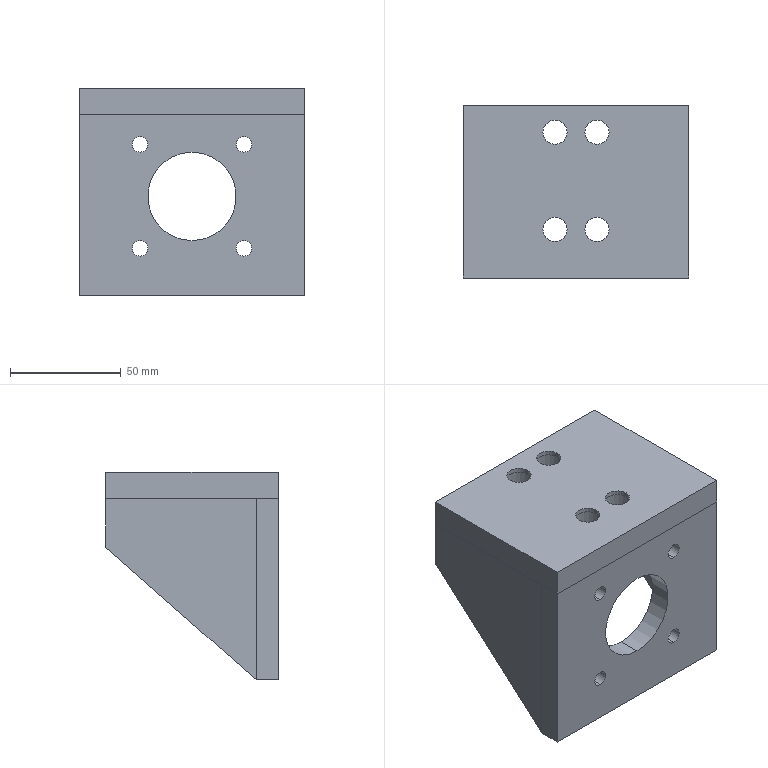Part | SolidWorks | features BaseBody 4 | 4 solids | 54 faces | box 102 x 78 x 94 mm | volume 211743 mm3 | plane 28 | cylinder 26 | commonest cylinder face diameters 7 x8 11 x8 17 x8 40 x2
STEP:
#1=CARTESIAN_POINT('',(23.5,-29.,-10.));
#2=VERTEX_POINT('',#1);
#3=CARTESIAN_POINT('',(23.5,-29.,-17.));
#4=VERTEX_POINT('',#3);
#5=CARTESIAN_POINT('',(23.5,-29.,-13.5));
#6=DIRECTION('',(0.,-1.,0.));
#7=DIRECTION('',(0.,0.,-1.));
#8=AXIS2_PLACEMENT_3D('',#5,#6,#7);
#9=CIRCLE('',#8,3.5);
#10=EDGE_CURVE('',#2,#4,#9,.T.);
#11=ORIENTED_EDGE('',*,*,#10,.F.);
#12=CARTESIAN_POINT('',(23.5,-39.,-10.));
#13=VERTEX_POINT('',#12);
#14=CARTESIAN_POINT('',(23.5,-29.,-10.));
#15=DIRECTION('',(0.,-1.,0.));
#16=VECTOR('',#15,1000.);
#17=LINE('',#14,#16);
#18=EDGE_CURVE('',#2,#13,#17,.T.);
#19=ORIENTED_EDGE('',*,*,#18,.T.);
#20=CARTESIAN_POINT('',(23.5,-39.,-17.));
#21=VERTEX_POINT('',#20);
#22=CARTESIAN_POINT('',(23.5,-39.,-13.5));
#23=DIRECTION('',(0.,-1.,0.));
#24=DIRECTION('',(0.,0.,-1.));
#25=AXIS2_PLACEMENT_3D('',#22,#23,#24);
#26=CIRCLE('',#25,3.5);
#27=EDGE_CURVE('',#13,#21,#26,.T.);
#28=ORIENTED_EDGE('',*,*,#27,.T.);
#29=CARTESIAN_POINT('',(23.5,-29.,-17.));
#30=DIRECTION('',(0.,-1.,0.));
#31=VECTOR('',#30,1000.);
#32=LINE('',#29,#31);
#33=EDGE_CURVE('',#4,#21,#32,.T.);
#34=ORIENTED_EDGE('',*,*,#33,.F.);
#35=EDGE_LOOP('',(#11,#19,#28,#34));
#36=FACE_OUTER_BOUND('',#35,.T.);
#37=CARTESIAN_POINT('',(23.5,-29.,-13.5));
#38=DIRECTION('',(0.,-1.,0.));
#39=DIRECTION('',(0.,0.,-1.));
#40=AXIS2_PLACEMENT_3D('',#37,#38,#39);
#41=CYLINDRICAL_SURFACE('',#40,3.5);
#42=ADVANCED_FACE('',(#36),#41,.F.);
#43=CARTESIAN_POINT('',(-23.5,-29.,-10.));
#44=VERTEX_POINT('',#43);
#45=CARTESIAN_POINT('',(-23.5,-29.,-17.));
#46=VERTEX_POINT('',#45);
#47=CARTESIAN_POINT('',(-23.5,-29.,-13.5));
#48=DIRECTION('',(0.,-1.,0.));
#49=DIRECTION('',(0.,0.,-1.));
#50=AXIS2_PLACEMENT_3D('',#47,#48,#49);
#51=CIRCLE('',#50,3.5);
#52=EDGE_CURVE('',#44,#46,#51,.T.);
#53=ORIENTED_EDGE('',*,*,#52,.F.);
#54=CARTESIAN_POINT('',(-23.5,-39.,-10.));
#55=VERTEX_POINT('',#54);
#56=CARTESIAN_POINT('',(-23.5,-29.,-10.));
#57=DIRECTION('',(0.,-1.,0.));
#58=VECTOR('',#57,1000.);
#59=LINE('',#56,#58);
#60=EDGE_CURVE('',#44,#55,#59,.T.);
#61=ORIENTED_EDGE('',*,*,#60,.T.);
#62=CARTESIAN_POINT('',(-23.5,-39.,-17.));
#63=VERTEX_POINT('',#62);
#64=CARTESIAN_POINT('',(-23.5,-39.,-13.5));
#65=DIRECTION('',(0.,-1.,0.));
#66=DIRECTION('',(0.,0.,-1.));
#67=AXIS2_PLACEMENT_3D('',#64,#65,#66);
#68=CIRCLE('',#67,3.5);
#69=EDGE_CURVE('',#55,#63,#68,.T.);
#70=ORIENTED_EDGE('',*,*,#69,.T.);
#71=CARTESIAN_POINT('',(-23.5,-29.,-17.));
#72=DIRECTION('',(0.,-1.,0.));
#73=VECTOR('',#72,1000.);
#74=LINE('',#71,#73);
#75=EDGE_CURVE('',#46,#63,#74,.T.);
#76=ORIENTED_EDGE('',*,*,#75,.F.);
#77=EDGE_LOOP('',(#53,#61,#70,#76));
#78=FACE_OUTER_BOUND('',#77,.T.);
#79=CARTESIAN_POINT('',(-23.5,-29.,-13.5));
#80=DIRECTION('',(0.,-1.,0.));
#81=DIRECTION('',(0.,0.,-1.));
#82=AXIS2_PLACEMENT_3D('',#79,#80,#81);
#83=CYLINDRICAL_SURFACE('',#82,3.5);
#84=ADVANCED_FACE('',(#78),#83,.F.);
#85=CARTESIAN_POINT('',(-23.5,-29.,-57.));
#86=VERTEX_POINT('',#85);
#87=CARTESIAN_POINT('',(-23.5,-29.,-64.));
#88=VERTEX_POINT('',#87);
#89=CARTESIAN_POINT('',(-23.5,-29.,-60.5));
#90=DIRECTION('',(0.,-1.,0.));
#91=DIRECTION('',(0.,0.,-1.));
#92=AXIS2_PLACEMENT_3D('',#89,#90,#91);
#93=CIRCLE('',#92,3.5);
#94=EDGE_CURVE('',#86,#88,#93,.T.);
#95=ORIENTED_EDGE('',*,*,#94,.F.);
#96=CARTESIAN_POINT('',(-23.5,-39.,-57.));
#97=VERTEX_POINT('',#96);
#98=CARTESIAN_POINT('',(-23.5,-29.,-57.));
#99=DIRECTION('',(0.,-1.,0.));
#100=VECTOR('',#99,1000.);
#101=LINE('',#98,#100);
#102=EDGE_CURVE('',#86,#97,#101,.T.);
#103=ORIENTED_EDGE('',*,*,#102,.T.);
#104=CARTESIAN_POINT('',(-23.5,-39.,-64.));
#105=VERTEX_POINT('',#104);
#106=CARTESIAN_POINT('',(-23.5,-39.,-60.5));
#107=DIRECTION('',(0.,-1.,0.));
#108=DIRECTION('',(0.,0.,-1.));
#109=AXIS2_PLACEMENT_3D('',#106,#107,#108);
#110=CIRCLE('',#109,3.5);
#111=EDGE_CURVE('',#97,#105,#110,.T.);
#112=ORIENTED_EDGE('',*,*,#111,.T.);
#113=CARTESIAN_POINT('',(-23.5,-29.,-64.));
#114=DIRECTION('',(0.,-1.,0.));
#115=VECTOR('',#114,1000.);
#116=LINE('',#113,#115);
#117=EDGE_CURVE('',#88,#105,#116,.T.);
#118=ORIENTED_EDGE('',*,*,#117,.F.);
#119=EDGE_LOOP('',(#95,#103,#112,#118));
#120=FACE_OUTER_BOUND('',#119,.T.);
#121=CARTESIAN_POINT('',(-23.5,-29.,-60.5));
#122=DIRECTION('',(0.,-1.,0.));
#123=DIRECTION('',(0.,0.,-1.));
#124=AXIS2_PLACEMENT_3D('',#121,#122,#123);
#125=CYLINDRICAL_SURFACE('',#124,3.5);
#126=ADVANCED_FACE('',(#120),#125,.F.);
#127=CARTESIAN_POINT('',(23.5,-29.,-57.));
#128=VERTEX_POINT('',#127);
#129=CARTESIAN_POINT('',(23.5,-29.,-64.));
#130=VERTEX_POINT('',#129);
#131=CARTESIAN_POINT('',(23.5,-29.,-60.5));
#132=DIRECTION('',(0.,-1.,0.));
#133=DIRECTION('',(0.,0.,-1.));
#134=AXIS2_PLACEMENT_3D('',#131,#132,#133);
#135=CIRCLE('',#134,3.5);
#136=EDGE_CURVE('',#128,#130,#135,.T.);
#137=ORIENTED_EDGE('',*,*,#136,.F.);
#138=CARTESIAN_POINT('',(23.5,-39.,-57.));
#139=VERTEX_POINT('',#138);
#140=CARTESIAN_POINT('',(23.5,-29.,-57.));
#141=DIRECTION('',(0.,-1.,0.));
#142=VECTOR('',#141,1000.);
#143=LINE('',#140,#142);
#144=EDGE_CURVE('',#128,#139,#143,.T.);
#145=ORIENTED_EDGE('',*,*,#144,.T.);
#146=CARTESIAN_POINT('',(23.5,-39.,-64.));
#147=VERTEX_POINT('',#146);
#148=CARTESIAN_POINT('',(23.5,-39.,-60.5));
#149=DIRECTION('',(0.,-1.,0.));
#150=DIRECTION('',(0.,0.,-1.));
#151=AXIS2_PLACEMENT_3D('',#148,#149,#150);
#152=CIRCLE('',#151,3.5);
#153=EDGE_CURVE('',#139,#147,#152,.T.);
#154=ORIENTED_EDGE('',*,*,#153,.T.);
#155=CARTESIAN_POINT('',(23.5,-29.,-64.));
#156=DIRECTION('',(0.,-1.,0.));
#157=VECTOR('',#156,1000.);
#158=LINE('',#155,#157);
#159=EDGE_CURVE('',#130,#147,#158,.T.);
#160=ORIENTED_EDGE('',*,*,#159,.F.);
#161=EDGE_LOOP('',(#137,#145,#154,#160));
#162=FACE_OUTER_BOUND('',#161,.T.);
#163=CARTESIAN_POINT('',(23.5,-29.,-60.5));
#164=DIRECTION('',(0.,-1.,0.));
#165=DIRECTION('',(0.,0.,-1.));
#166=AXIS2_PLACEMENT_3D('',#163,#164,#165);
#167=CYLINDRICAL_SURFACE('',#166,3.5);
#168=ADVANCED_FACE('',(#162),#167,.F.);
#169=CARTESIAN_POINT('',(0.,-29.,-17.));
#170=VERTEX_POINT('',#169);
#171=CARTESIAN_POINT('',(0.,-29.,-57.));
#172=VERTEX_POINT('',#171);
#173=CARTESIAN_POINT('',(0.,-29.,-37.));
#174=DIRECTION('',(0.,-1.,0.));
#175=DIRECTION('',(0.,0.,-1.));
#176=AXIS2_PLACEMENT_3D('',#173,#174,#175);
#177=CIRCLE('',#176,20.);
#178=EDGE_CURVE('',#170,#172,#177,.T.);
#179=ORIENTED_EDGE('',*,*,#178,.F.);
#180=CARTESIAN_POINT('',(0.,-39.,-17.));
#181=VERTEX_POINT('',#180);
#182=CARTESIAN_POINT('',(0.,-29.,-17.));
#183=DIRECTION('',(0.,-1.,0.));
#184=VECTOR('',#183,1000.);
#185=LINE('',#182,#184);
#186=EDGE_CURVE('',#170,#181,#185,.T.);
#187=ORIENTED_EDGE('',*,*,#186,.T.);
#188=CARTESIAN_POINT('',(0.,-39.,-57.));
#189=VERTEX_POINT('',#188);
#190=CARTESIAN_POINT('',(0.,-39.,-37.));
#191=DIRECTION('',(0.,-1.,0.));
#192=DIRECTION('',(0.,0.,-1.));
#193=AXIS2_PLACEMENT_3D('',#190,#191,#192);
#194=CIRCLE('',#193,20.);
#195=EDGE_CURVE('',#181,#189,#194,.T.);
#196=ORIENTED_EDGE('',*,*,#195,.T.);
#197=CARTESIAN_POINT('',(0.,-29.,-57.));
#198=DIRECTION('',(0.,-1.,0.));
#199=VECTOR('',#198,1000.);
#200=LINE('',#197,#199);
#201=EDGE_CURVE('',#172,#189,#200,.T.);
#202=ORIENTED_EDGE('',*,*,#201,.F.);
#203=EDGE_LOOP('',(#179,#187,#196,#202));
#204=FACE_OUTER_BOUND('',#203,.T.);
#205=CARTESIAN_POINT('',(0.,-29.,-37.));
#206=DIRECTION('',(0.,-1.,0.));
#207=DIRECTION('',(0.,0.,-1.));
#208=AXIS2_PLACEMENT_3D('',#205,#206,#207);
#209=CYLINDRICAL_SURFACE('',#208,20.);
#210=ADVANCED_FACE('',(#204),#209,.F.);
#211=CARTESIAN_POINT('',(51.,-39.,-82.));
#212=VERTEX_POINT('',#211);
#213=CARTESIAN_POINT('',(51.,-39.,0.));
#214=VERTEX_POINT('',#213);
#215=CARTESIAN_POINT('',(51.,-39.,0.));
#216=DIRECTION('',(0.,0.,1.));
#217=VECTOR('',#216,1000.);
#218=LINE('',#215,#217);
#219=EDGE_CURVE('',#212,#214,#218,.T.);
#220=ORIENTED_EDGE('',*,*,#219,.F.);
#221=CARTESIAN_POINT('',(51.,-29.,-82.));
#222=VERTEX_POINT('',#221);
#223=CARTESIAN_POINT('',(51.,-29.,-82.));
#224=DIRECTION('',(0.,-1.,0.));
#225=VECTOR('',#224,1000.);
#226=LINE('',#223,#225);
#227=EDGE_CURVE('',#222,#212,#226,.T.);
#228=ORIENTED_EDGE('',*,*,#227,.F.);
#229=CARTESIAN_POINT('',(51.,-29.,0.));
#230=VERTEX_POINT('',#229);
#231=CARTESIAN_POINT('',(51.,-29.,0.));
#232=DIRECTION('',(0.,0.,1.));
#233=VECTOR('',#232,1000.);
#234=LINE('',#231,#233);
#235=EDGE_CURVE('',#222,#230,#234,.T.);
#236=ORIENTED_EDGE('',*,*,#235,.T.);
#237=CARTESIAN_POINT('',(51.,-29.,0.));
#238=DIRECTION('',(0.,-1.,0.));
#239=VECTOR('',#238,1000.);
#240=LINE('',#237,#239);
#241=EDGE_CURVE('',#230,#214,#240,.T.);
#242=ORIENTED_EDGE('',*,*,#241,.T.);
#243=EDGE_LOOP('',(#220,#228,#236,#242));
#244=FACE_OUTER_BOUND('',#243,.T.);
#245=CARTESIAN_POINT('',(51.,-29.,0.));
#246=DIRECTION('',(1.,0.,0.));
#247=DIRECTION('',(0.,0.,-1.));
#248=AXIS2_PLACEMENT_3D('',#245,#246,#247);
#249=PLANE('',#248);
#250=ADVANCED_FACE('',(#244),#249,.T.);
#251=CARTESIAN_POINT('',(-51.,-39.,-82.));
#252=VERTEX_POINT('',#251);
#253=CARTESIAN_POINT('',(51.,-39.,-82.));
#254=DIRECTION('',(1.,0.,0.));
#255=VECTOR('',#254,1000.);
#256=LINE('',#253,#255);
#257=EDGE_CURVE('',#252,#212,#256,.T.);
#258=ORIENTED_EDGE('',*,*,#257,.F.);
#259=CARTESIAN_POINT('',(-51.,-29.,-82.));
#260=VERTEX_POINT('',#259);
#261=CARTESIAN_POINT('',(-51.,-29.,-82.));
#262=DIRECTION('',(0.,-1.,0.));
#263=VECTOR('',#262,1000.);
#264=LINE('',#261,#263);
#265=EDGE_CURVE('',#260,#252,#264,.T.);
#266=ORIENTED_EDGE('',*,*,#265,.F.);
#267=CARTESIAN_POINT('',(51.,-29.,-82.));
#268=DIRECTION('',(1.,0.,0.));
#269=VECTOR('',#268,1000.);
#270=LINE('',#267,#269);
#271=EDGE_CURVE('',#260,#222,#270,.T.);
#272=ORIENTED_EDGE('',*,*,#271,.T.);
#273=ORIENTED_EDGE('',*,*,#227,.T.);
#274=EDGE_LOOP('',(#258,#266,#272,#273));
#275=FACE_OUTER_BOUND('',#274,.T.);
#276=CARTESIAN_POINT('',(51.,-29.,-82.));
#277=DIRECTION('',(0.,0.,-1.));
#278=DIRECTION('',(-1.,0.,0.));
#279=AXIS2_PLACEMENT_3D('',#276,#277,#278);
#280=PLANE('',#279);
#281=ADVANCED_FACE('',(#275),#280,.T.);
#282=CARTESIAN_POINT('',(-51.,-39.,0.));
#283=VERTEX_POINT('',#282);
#284=CARTESIAN_POINT('',(-51.,-39.,0.));
#285=DIRECTION('',(0.,0.,-1.));
#286=VECTOR('',#285,1000.);
#287=LINE('',#284,#286);
#288=EDGE_CURVE('',#283,#252,#287,.T.);
#289=ORIENTED_EDGE('',*,*,#288,.F.);
#290=CARTESIAN_POINT('',(-51.,-29.,0.));
#291=VERTEX_POINT('',#290);
#292=CARTESIAN_POINT('',(-51.,-29.,0.));
#293=DIRECTION('',(0.,-1.,0.));
#294=VECTOR('',#293,1000.);
#295=LINE('',#292,#294);
#296=EDGE_CURVE('',#291,#283,#295,.T.);
#297=ORIENTED_EDGE('',*,*,#296,.F.);
#298=CARTESIAN_POINT('',(-51.,-29.,0.));
#299=DIRECTION('',(0.,0.,-1.));
#300=VECTOR('',#299,1000.);
#301=LINE('',#298,#300);
#302=EDGE_CURVE('',#291,#260,#301,.T.);
#303=ORIENTED_EDGE('',*,*,#302,.T.);
#304=ORIENTED_EDGE('',*,*,#265,.T.);
#305=EDGE_LOOP('',(#289,#297,#303,#304));
#306=FACE_OUTER_BOUND('',#305,.T.);
#307=CARTESIAN_POINT('',(-51.,-29.,0.));
#308=DIRECTION('',(-1.,0.,0.));
#309=DIRECTION('',(0.,0.,1.));
#310=AXIS2_PLACEMENT_3D('',#307,#308,#309);
#311=PLANE('',#310);
#312=ADVANCED_FACE('',(#306),#311,.T.);
#313=CARTESIAN_POINT('',(51.,-39.,0.));
#314=DIRECTION('',(-1.,0.,0.));
#315=VECTOR('',#314,1000.);
#316=LINE('',#313,#315);
#317=EDGE_CURVE('',#214,#283,#316,.T.);
#318=ORIENTED_EDGE('',*,*,#317,.F.);
#319=ORIENTED_EDGE('',*,*,#241,.F.);
#320=CARTESIAN_POINT('',(51.,-29.,0.));
#321=DIRECTION('',(-1.,0.,0.));
#322=VECTOR('',#321,1000.);
#323=LINE('',#320,#322);
#324=EDGE_CURVE('',#230,#291,#323,.T.);
#325=ORIENTED_EDGE('',*,*,#324,.T.);
#326=ORIENTED_EDGE('',*,*,#296,.T.);
#327=EDGE_LOOP('',(#318,#319,#325,#326));
#328=FACE_OUTER_BOUND('',#327,.T.);
#329=CARTESIAN_POINT('',(51.,-29.,0.));
#330=DIRECTION('',(0.,0.,1.));
#331=DIRECTION('',(1.,0.,0.));
#332=AXIS2_PLACEMENT_3D('',#329,#330,#331);
#333=PLANE('',#332);
#334=ADVANCED_FACE('',(#328),#333,.T.);
#335=CARTESIAN_POINT('',(23.5,-29.,-13.5));
#336=DIRECTION('',(0.,-1.,0.));
#337=DIRECTION('',(0.,0.,-1.));
#338=AXIS2_PLACEMENT_3D('',#335,#336,#337);
#339=CIRCLE('',#338,3.5);
#340=EDGE_CURVE('',#4,#2,#339,.T.);
#341=ORIENTED_EDGE('',*,*,#340,.T.);
#342=ORIENTED_EDGE('',*,*,#10,.T.);
#343=EDGE_LOOP('',(#341,#342));
#344=FACE_BOUND('',#343,.T.);
#345=CARTESIAN_POINT('',(-23.5,-29.,-13.5));
#346=DIRECTION('',(0.,-1.,0.));
#347=DIRECTION('',(0.,0.,-1.));
#348=AXIS2_PLACEMENT_3D('',#345,#346,#347);
#349=CIRCLE('',#348,3.5);
#350=EDGE_CURVE('',#46,#44,#349,.T.);
#351=ORIENTED_EDGE('',*,*,#350,.T.);
#352=ORIENTED_EDGE('',*,*,#52,.T.);
#353=EDGE_LOOP('',(#351,#352));
#354=FACE_BOUND('',#353,.T.);
#355=CARTESIAN_POINT('',(-23.5,-29.,-60.5));
#356=DIRECTION('',(0.,-1.,0.));
#357=DIRECTION('',(0.,0.,-1.));
#358=AXIS2_PLACEMENT_3D('',#355,#356,#357);
#359=CIRCLE('',#358,3.5);
#360=EDGE_CURVE('',#88,#86,#359,.T.);
#361=ORIENTED_EDGE('',*,*,#360,.T.);
#362=ORIENTED_EDGE('',*,*,#94,.T.);
#363=EDGE_LOOP('',(#361,#362));
#364=FACE_BOUND('',#363,.T.);
#365=CARTESIAN_POINT('',(23.5,-29.,-60.5));
#366=DIRECTION('',(0.,-1.,0.));
#367=DIRECTION('',(0.,0.,-1.));
#368=AXIS2_PLACEMENT_3D('',#365,#366,#367);
#369=CIRCLE('',#368,3.5);
#370=EDGE_CURVE('',#130,#128,#369,.T.);
#371=ORIENTED_EDGE('',*,*,#370,.T.);
#372=ORIENTED_EDGE('',*,*,#136,.T.);
#373=EDGE_LOOP('',(#371,#372));
#374=FACE_BOUND('',#373,.T.);
#375=CARTESIAN_POINT('',(0.,-29.,-37.));
#376=DIRECTION('',(0.,-1.,0.));
#377=DIRECTION('',(0.,0.,-1.));
#378=AXIS2_PLACEMENT_3D('',#375,#376,#377);
#379=CIRCLE('',#378,20.);
#380=EDGE_CURVE('',#172,#170,#379,.T.);
#381=ORIENTED_EDGE('',*,*,#380,.T.);
#382=ORIENTED_EDGE('',*,*,#178,.T.);
#383=EDGE_LOOP('',(#381,#382));
#384=FACE_BOUND('',#383,.T.);
#385=ORIENTED_EDGE('',*,*,#235,.F.);
#386=ORIENTED_EDGE('',*,*,#271,.F.);
#387=ORIENTED_EDGE('',*,*,#302,.F.);
#388=ORIENTED_EDGE('',*,*,#324,.F.);
#389=EDGE_LOOP('',(#385,#386,#387,#388));
#390=FACE_OUTER_BOUND('',#389,.T.);
#391=CARTESIAN_POINT('',(0.,-29.,0.));
#392=DIRECTION('',(0.,1.,0.));
#393=DIRECTION('',(0.,0.,1.));
#394=AXIS2_PLACEMENT_3D('',#391,#392,#393);
#395=PLANE('',#394);
#396=ADVANCED_FACE('',(#344,#354,#364,#374,#384,#390),#395,.T.);
#397=CARTESIAN_POINT('',(23.5,-39.,-13.5));
#398=DIRECTION('',(0.,-1.,0.));
#399=DIRECTION('',(0.,0.,-1.));
#400=AXIS2_PLACEMENT_3D('',#397,#398,#399);
#401=CIRCLE('',#400,3.5);
#402=EDGE_CURVE('',#21,#13,#401,.T.);
#403=ORIENTED_EDGE('',*,*,#402,.F.);
#404=ORIENTED_EDGE('',*,*,#27,.F.);
#405=EDGE_LOOP('',(#403,#404));
#406=FACE_BOUND('',#405,.T.);
#407=CARTESIAN_POINT('',(-23.5,-39.,-13.5));
#408=DIRECTION('',(0.,-1.,0.));
#409=DIRECTION('',(0.,0.,-1.));
#410=AXIS2_PLACEMENT_3D('',#407,#408,#409);
#411=CIRCLE('',#410,3.5);
#412=EDGE_CURVE('',#63,#55,#411,.T.);
#413=ORIENTED_EDGE('',*,*,#412,.F.);
#414=ORIENTED_EDGE('',*,*,#69,.F.);
#415=EDGE_LOOP('',(#413,#414));
#416=FACE_BOUND('',#415,.T.);
#417=CARTESIAN_POINT('',(-23.5,-39.,-60.5));
#418=DIRECTION('',(0.,-1.,0.));
#419=DIRECTION('',(0.,0.,-1.));
#420=AXIS2_PLACEMENT_3D('',#417,#418,#419);
#421=CIRCLE('',#420,3.5);
#422=EDGE_CURVE('',#105,#97,#421,.T.);
#423=ORIENTED_EDGE('',*,*,#422,.F.);
#424=ORIENTED_EDGE('',*,*,#111,.F.);
#425=EDGE_LOOP('',(#423,#424));
#426=FACE_BOUND('',#425,.T.);
#427=CARTESIAN_POINT('',(23.5,-39.,-60.5));
#428=DIRECTION('',(0.,-1.,0.));
#429=DIRECTION('',(0.,0.,-1.));
#430=AXIS2_PLACEMENT_3D('',#427,#428,#429);
#431=CIRCLE('',#430,3.5);
#432=EDGE_CURVE('',#147,#139,#431,.T.);
#433=ORIENTED_EDGE('',*,*,#432,.F.);
#434=ORIENTED_EDGE('',*,*,#153,.F.);
#435=EDGE_LOOP('',(#433,#434));
#436=FACE_BOUND('',#435,.T.);
#437=CARTESIAN_POINT('',(0.,-39.,-37.));
#438=DIRECTION('',(0.,-1.,0.));
#439=DIRECTION('',(0.,0.,-1.));
#440=AXIS2_PLACEMENT_3D('',#437,#438,#439);
#441=CIRCLE('',#440,20.);
#442=EDGE_CURVE('',#189,#181,#441,.T.);
#443=ORIENTED_EDGE('',*,*,#442,.F.);
#444=ORIENTED_EDGE('',*,*,#195,.F.);
#445=EDGE_LOOP('',(#443,#444));
#446=FACE_BOUND('',#445,.T.);
#447=ORIENTED_EDGE('',*,*,#219,.T.);
#448=ORIENTED_EDGE('',*,*,#317,.T.);
#449=ORIENTED_EDGE('',*,*,#288,.T.);
#450=ORIENTED_EDGE('',*,*,#257,.T.);
#451=EDGE_LOOP('',(#447,#448,#449,#450));
#452=FACE_OUTER_BOUND('',#451,.T.);
#453=CARTESIAN_POINT('',(0.,-39.,0.));
#454=DIRECTION('',(0.,1.,0.));
#455=DIRECTION('',(0.,0.,1.));
#456=AXIS2_PLACEMENT_3D('',#453,#454,#455);
#457=PLANE('',#456);
#458=ADVANCED_FACE('',(#406,#416,#426,#436,#446,#452),#457,.F.);
#459=ORIENTED_EDGE('',*,*,#186,.F.);
#460=ORIENTED_EDGE('',*,*,#380,.F.);
#461=ORIENTED_EDGE('',*,*,#201,.T.);
#462=ORIENTED_EDGE('',*,*,#442,.T.);
#463=EDGE_LOOP('',(#459,#460,#461,#462));
#464=FACE_OUTER_BOUND('',#463,.T.);
#465=CARTESIAN_POINT('',(0.,-29.,-37.));
#466=DIRECTION('',(0.,-1.,0.));
#467=DIRECTION('',(0.,0.,-1.));
#468=AXIS2_PLACEMENT_3D('',#465,#466,#467);
#469=CYLINDRICAL_SURFACE('',#468,20.);
#470=ADVANCED_FACE('',(#464),#469,.F.);
#471=ORIENTED_EDGE('',*,*,#144,.F.);
#472=ORIENTED_EDGE('',*,*,#370,.F.);
#473=ORIENTED_EDGE('',*,*,#159,.T.);
#474=ORIENTED_EDGE('',*,*,#432,.T.);
#475=EDGE_LOOP('',(#471,#472,#473,#474));
#476=FACE_OUTER_BOUND('',#475,.T.);
#477=CARTESIAN_POINT('',(23.5,-29.,-60.5));
#478=DIRECTION('',(0.,-1.,0.));
#479=DIRECTION('',(0.,0.,-1.));
#480=AXIS2_PLACEMENT_3D('',#477,#478,#479);
#481=CYLINDRICAL_SURFACE('',#480,3.5);
#482=ADVANCED_FACE('',(#476),#481,.F.);
#483=ORIENTED_EDGE('',*,*,#102,.F.);
#484=ORIENTED_EDGE('',*,*,#360,.F.);
#485=ORIENTED_EDGE('',*,*,#117,.T.);
#486=ORIENTED_EDGE('',*,*,#422,.T.);
#487=EDGE_LOOP('',(#483,#484,#485,#486));
#488=FACE_OUTER_BOUND('',#487,.T.);
#489=CARTESIAN_POINT('',(-23.5,-29.,-60.5));
#490=DIRECTION('',(0.,-1.,0.));
#491=DIRECTION('',(0.,0.,-1.));
#492=AXIS2_PLACEMENT_3D('',#489,#490,#491);
#493=CYLINDRICAL_SURFACE('',#492,3.5);
#494=ADVANCED_FACE('',(#488),#493,.F.);
#495=ORIENTED_EDGE('',*,*,#60,.F.);
#496=ORIENTED_EDGE('',*,*,#350,.F.);
#497=ORIENTED_EDGE('',*,*,#75,.T.);
#498=ORIENTED_EDGE('',*,*,#412,.T.);
#499=EDGE_LOOP('',(#495,#496,#497,#498));
#500=FACE_OUTER_BOUND('',#499,.T.);
#501=CARTESIAN_POINT('',(-23.5,-29.,-13.5));
#502=DIRECTION('',(0.,-1.,0.));
#503=DIRECTION('',(0.,0.,-1.));
#504=AXIS2_PLACEMENT_3D('',#501,#502,#503);
#505=CYLINDRICAL_SURFACE('',#504,3.5);
#506=ADVANCED_FACE('',(#500),#505,.F.);
#507=ORIENTED_EDGE('',*,*,#18,.F.);
#508=ORIENTED_EDGE('',*,*,#340,.F.);
#509=ORIENTED_EDGE('',*,*,#33,.T.);
#510=ORIENTED_EDGE('',*,*,#402,.T.);
#511=EDGE_LOOP('',(#507,#508,#509,#510));
#512=FACE_OUTER_BOUND('',#511,.T.);
#513=CARTESIAN_POINT('',(23.5,-29.,-13.5));
#514=DIRECTION('',(0.,-1.,0.));
#515=DIRECTION('',(0.,0.,-1.));
#516=AXIS2_PLACEMENT_3D('',#513,#514,#515);
#517=CYLINDRICAL_SURFACE('',#516,3.5);
#518=ADVANCED_FACE('',(#512),#517,.F.);
#519=CLOSED_SHELL('',(#42,#84,#126,#168,#210,#250,#281,#312,#334,#396,#458,#470,#482,#494,#506,#518));
#520=MANIFOLD_SOLID_BREP('',#519);
#521=CARTESIAN_POINT('',(51.,39.,0.));
#522=VERTEX_POINT('',#521);
#523=CARTESIAN_POINT('',(51.,-29.,0.));
#524=VERTEX_POINT('',#523);
#525=CARTESIAN_POINT('',(51.,-29.,0.));
#526=DIRECTION('',(0.,-1.,0.));
#527=VECTOR('',#526,1000.);
#528=LINE('',#525,#527);
#529=EDGE_CURVE('',#522,#524,#528,.T.);
#530=ORIENTED_EDGE('',*,*,#529,.F.);
#531=CARTESIAN_POINT('',(43.,39.,0.));
#532=VERTEX_POINT('',#531);
#533=CARTESIAN_POINT('',(43.,39.,0.));
#534=DIRECTION('',(1.,0.,0.));
#535=VECTOR('',#534,1000.);
#536=LINE('',#533,#535);
#537=EDGE_CURVE('',#532,#522,#536,.T.);
#538=ORIENTED_EDGE('',*,*,#537,.F.);
#539=CARTESIAN_POINT('',(43.,-29.,0.));
#540=VERTEX_POINT('',#539);
#541=CARTESIAN_POINT('',(43.,-29.,0.));
#542=DIRECTION('',(0.,-1.,0.));
#543=VECTOR('',#542,1000.);
#544=LINE('',#541,#543);
#545=EDGE_CURVE('',#532,#540,#544,.T.);
#546=ORIENTED_EDGE('',*,*,#545,.T.);
#547=CARTESIAN_POINT('',(43.,-29.,0.));
#548=DIRECTION('',(1.,0.,0.));
#549=VECTOR('',#548,1000.);
#550=LINE('',#547,#549);
#551=EDGE_CURVE('',#540,#524,#550,.T.);
#552=ORIENTED_EDGE('',*,*,#551,.T.);
#553=EDGE_LOOP('',(#530,#538,#546,#552));
#554=FACE_OUTER_BOUND('',#553,.T.);
#555=CARTESIAN_POINT('',(43.,-29.,0.));
#556=DIRECTION('',(0.,0.,1.));
#557=DIRECTION('',(1.,0.,0.));
#558=AXIS2_PLACEMENT_3D('',#555,#556,#557);
#559=PLANE('',#558);
#560=ADVANCED_FACE('',(#554),#559,.T.);
#561=CARTESIAN_POINT('',(51.,39.,-22.));
#562=VERTEX_POINT('',#561);
#563=CARTESIAN_POINT('',(51.,39.,0.));
#564=DIRECTION('',(0.,0.,1.));
#565=VECTOR('',#564,1000.);
#566=LINE('',#563,#565);
#567=EDGE_CURVE('',#562,#522,#566,.T.);
#568=ORIENTED_EDGE('',*,*,#567,.F.);
#569=CARTESIAN_POINT('',(43.,39.,-22.));
#570=VERTEX_POINT('',#569);
#571=CARTESIAN_POINT('',(43.,39.,-22.));
#572=DIRECTION('',(1.,0.,0.));
#573=VECTOR('',#572,1000.);
#574=LINE('',#571,#573);
#575=EDGE_CURVE('',#570,#562,#574,.T.);
#576=ORIENTED_EDGE('',*,*,#575,.F.);
#577=CARTESIAN_POINT('',(43.,39.,0.));
#578=DIRECTION('',(0.,0.,1.));
#579=VECTOR('',#578,1000.);
#580=LINE('',#577,#579);
#581=EDGE_CURVE('',#570,#532,#580,.T.);
#582=ORIENTED_EDGE('',*,*,#581,.T.);
#583=ORIENTED_EDGE('',*,*,#537,.T.);
#584=EDGE_LOOP('',(#568,#576,#582,#583));
#585=FACE_OUTER_BOUND('',#584,.T.);
#586=CARTESIAN_POINT('',(43.,39.,0.));
#587=DIRECTION('',(0.,1.,0.));
#588=DIRECTION('',(0.,0.,1.));
#589=AXIS2_PLACEMENT_3D('',#586,#587,#588);
#590=PLANE('',#589);
#591=ADVANCED_FACE('',(#585),#590,.T.);
#592=CARTESIAN_POINT('',(51.,-29.,-82.));
#593=VERTEX_POINT('',#592);
#594=CARTESIAN_POINT('',(51.,39.,-22.));
#595=DIRECTION('',(0.,0.7498,0.6616));
#596=VECTOR('',#595,1000.);
#597=LINE('',#594,#596);
#598=EDGE_CURVE('',#593,#562,#597,.T.);
#599=ORIENTED_EDGE('',*,*,#598,.F.);
#600=CARTESIAN_POINT('',(43.,-29.,-82.));
#601=VERTEX_POINT('',#600);
#602=CARTESIAN_POINT('',(43.,-29.,-82.));
#603=DIRECTION('',(1.,0.,0.));
#604=VECTOR('',#603,1000.);
#605=LINE('',#602,#604);
#606=EDGE_CURVE('',#601,#593,#605,.T.);
#607=ORIENTED_EDGE('',*,*,#606,.F.);
#608=CARTESIAN_POINT('',(43.,39.,-22.));
#609=DIRECTION('',(0.,0.7498,0.6616));
#610=VECTOR('',#609,1000.);
#611=LINE('',#608,#610);
#612=EDGE_CURVE('',#601,#570,#611,.T.);
#613=ORIENTED_EDGE('',*,*,#612,.T.);
#614=ORIENTED_EDGE('',*,*,#575,.T.);
#615=EDGE_LOOP('',(#599,#607,#613,#614));
#616=FACE_OUTER_BOUND('',#615,.T.);
#617=CARTESIAN_POINT('',(43.,39.,-22.));
#618=DIRECTION('',(0.,0.6616,-0.7498));
#619=DIRECTION('',(0.,0.7498,0.6616));
#620=AXIS2_PLACEMENT_3D('',#617,#618,#619);
#621=PLANE('',#620);
#622=ADVANCED_FACE('',(#616),#621,.T.);
#623=CARTESIAN_POINT('',(51.,-29.,-82.));
#624=DIRECTION('',(0.,0.,-1.));
#625=VECTOR('',#624,1000.);
#626=LINE('',#623,#625);
#627=EDGE_CURVE('',#524,#593,#626,.T.);
#628=ORIENTED_EDGE('',*,*,#627,.F.);
#629=ORIENTED_EDGE('',*,*,#551,.F.);
#630=CARTESIAN_POINT('',(43.,-29.,-82.));
#631=DIRECTION('',(0.,0.,-1.));
#632=VECTOR('',#631,1000.);
#633=LINE('',#630,#632);
#634=EDGE_CURVE('',#540,#601,#633,.T.);
#635=ORIENTED_EDGE('',*,*,#634,.T.);
#636=ORIENTED_EDGE('',*,*,#606,.T.);
#637=EDGE_LOOP('',(#628,#629,#635,#636));
#638=FACE_OUTER_BOUND('',#637,.T.);
#639=CARTESIAN_POINT('',(43.,-29.,-82.));
#640=DIRECTION('',(0.,-1.,0.));
#641=DIRECTION('',(0.,0.,-1.));
#642=AXIS2_PLACEMENT_3D('',#639,#640,#641);
#643=PLANE('',#642);
#644=ADVANCED_FACE('',(#638),#643,.T.);
#645=ORIENTED_EDGE('',*,*,#545,.F.);
#646=ORIENTED_EDGE('',*,*,#581,.F.);
#647=ORIENTED_EDGE('',*,*,#612,.F.);
#648=ORIENTED_EDGE('',*,*,#634,.F.);
#649=EDGE_LOOP('',(#645,#646,#647,#648));
#650=FACE_OUTER_BOUND('',#649,.T.);
#651=CARTESIAN_POINT('',(43.,0.,0.));
#652=DIRECTION('',(-1.,0.,0.));
#653=DIRECTION('',(0.,0.,1.));
#654=AXIS2_PLACEMENT_3D('',#651,#652,#653);
#655=PLANE('',#654);
#656=ADVANCED_FACE('',(#650),#655,.T.);
#657=ORIENTED_EDGE('',*,*,#529,.T.);
#658=ORIENTED_EDGE('',*,*,#627,.T.);
#659=ORIENTED_EDGE('',*,*,#598,.T.);
#660=ORIENTED_EDGE('',*,*,#567,.T.);
#661=EDGE_LOOP('',(#657,#658,#659,#660));
#662=FACE_OUTER_BOUND('',#661,.T.);
#663=CARTESIAN_POINT('',(51.,0.,0.));
#664=DIRECTION('',(-1.,0.,0.));
#665=DIRECTION('',(0.,0.,1.));
#666=AXIS2_PLACEMENT_3D('',#663,#664,#665);
#667=PLANE('',#666);
#668=ADVANCED_FACE('',(#662),#667,.F.);
#669=CLOSED_SHELL('',(#560,#591,#622,#644,#656,#668));
#670=MANIFOLD_SOLID_BREP('',#669);
#671=CARTESIAN_POINT('',(-51.,39.,0.));
#672=VERTEX_POINT('',#671);
#673=CARTESIAN_POINT('',(-51.,-29.,0.));
#674=VERTEX_POINT('',#673);
#675=CARTESIAN_POINT('',(-51.,-29.,0.));
#676=DIRECTION('',(0.,-1.,0.));
#677=VECTOR('',#676,1000.);
#678=LINE('',#675,#677);
#679=EDGE_CURVE('',#672,#674,#678,.T.);
#680=ORIENTED_EDGE('',*,*,#679,.T.);
#681=CARTESIAN_POINT('',(-43.,-29.,0.));
#682=VERTEX_POINT('',#681);
#683=CARTESIAN_POINT('',(-43.,-29.,0.));
#684=DIRECTION('',(-1.,0.,0.));
#685=VECTOR('',#684,1000.);
#686=LINE('',#683,#685);
#687=EDGE_CURVE('',#682,#674,#686,.T.);
#688=ORIENTED_EDGE('',*,*,#687,.F.);
#689=CARTESIAN_POINT('',(-43.,39.,0.));
#690=VERTEX_POINT('',#689);
#691=CARTESIAN_POINT('',(-43.,-29.,0.));
#692=DIRECTION('',(0.,-1.,0.));
#693=VECTOR('',#692,1000.);
#694=LINE('',#691,#693);
#695=EDGE_CURVE('',#690,#682,#694,.T.);
#696=ORIENTED_EDGE('',*,*,#695,.F.);
#697=CARTESIAN_POINT('',(-43.,39.,0.));
#698=DIRECTION('',(-1.,0.,0.));
#699=VECTOR('',#698,1000.);
#700=LINE('',#697,#699);
#701=EDGE_CURVE('',#690,#672,#700,.T.);
#702=ORIENTED_EDGE('',*,*,#701,.T.);
#703=EDGE_LOOP('',(#680,#688,#696,#702));
#704=FACE_OUTER_BOUND('',#703,.T.);
#705=CARTESIAN_POINT('',(-43.,-29.,0.));
#706=DIRECTION('',(0.,0.,1.));
#707=DIRECTION('',(-1.,0.,0.));
#708=AXIS2_PLACEMENT_3D('',#705,#706,#707);
#709=PLANE('',#708);
#710=ADVANCED_FACE('',(#704),#709,.T.);
#711=CARTESIAN_POINT('',(-51.,39.,-22.));
#712=VERTEX_POINT('',#711);
#713=CARTESIAN_POINT('',(-51.,39.,0.));
#714=DIRECTION('',(0.,0.,1.));
#715=VECTOR('',#714,1000.);
#716=LINE('',#713,#715);
#717=EDGE_CURVE('',#712,#672,#716,.T.);
#718=ORIENTED_EDGE('',*,*,#717,.T.);
#719=ORIENTED_EDGE('',*,*,#701,.F.);
#720=CARTESIAN_POINT('',(-43.,39.,-22.));
#721=VERTEX_POINT('',#720);
#722=CARTESIAN_POINT('',(-43.,39.,0.));
#723=DIRECTION('',(0.,0.,1.));
#724=VECTOR('',#723,1000.);
#725=LINE('',#722,#724);
#726=EDGE_CURVE('',#721,#690,#725,.T.);
#727=ORIENTED_EDGE('',*,*,#726,.F.);
#728=CARTESIAN_POINT('',(-43.,39.,-22.));
#729=DIRECTION('',(-1.,0.,0.));
#730=VECTOR('',#729,1000.);
#731=LINE('',#728,#730);
#732=EDGE_CURVE('',#721,#712,#731,.T.);
#733=ORIENTED_EDGE('',*,*,#732,.T.);
#734=EDGE_LOOP('',(#718,#719,#727,#733));
#735=FACE_OUTER_BOUND('',#734,.T.);
#736=CARTESIAN_POINT('',(-43.,39.,0.));
#737=DIRECTION('',(0.,1.,0.));
#738=DIRECTION('',(0.,0.,1.));
#739=AXIS2_PLACEMENT_3D('',#736,#737,#738);
#740=PLANE('',#739);
#741=ADVANCED_FACE('',(#735),#740,.T.);
#742=CARTESIAN_POINT('',(-51.,-29.,-82.));
#743=VERTEX_POINT('',#742);
#744=CARTESIAN_POINT('',(-51.,39.,-22.));
#745=DIRECTION('',(0.,0.7498,0.6616));
#746=VECTOR('',#745,1000.);
#747=LINE('',#744,#746);
#748=EDGE_CURVE('',#743,#712,#747,.T.);
#749=ORIENTED_EDGE('',*,*,#748,.T.);
#750=ORIENTED_EDGE('',*,*,#732,.F.);
#751=CARTESIAN_POINT('',(-43.,-29.,-82.));
#752=VERTEX_POINT('',#751);
#753=CARTESIAN_POINT('',(-43.,39.,-22.));
#754=DIRECTION('',(0.,0.7498,0.6616));
#755=VECTOR('',#754,1000.);
#756=LINE('',#753,#755);
#757=EDGE_CURVE('',#752,#721,#756,.T.);
#758=ORIENTED_EDGE('',*,*,#757,.F.);
#759=CARTESIAN_POINT('',(-43.,-29.,-82.));
#760=DIRECTION('',(-1.,0.,0.));
#761=VECTOR('',#760,1000.);
#762=LINE('',#759,#761);
#763=EDGE_CURVE('',#752,#743,#762,.T.);
#764=ORIENTED_EDGE('',*,*,#763,.T.);
#765=EDGE_LOOP('',(#749,#750,#758,#764));
#766=FACE_OUTER_BOUND('',#765,.T.);
#767=CARTESIAN_POINT('',(-43.,39.,-22.));
#768=DIRECTION('',(0.,0.6616,-0.7498));
#769=DIRECTION('',(0.,0.7498,0.6616));
#770=AXIS2_PLACEMENT_3D('',#767,#768,#769);
#771=PLANE('',#770);
#772=ADVANCED_FACE('',(#766),#771,.T.);
#773=CARTESIAN_POINT('',(-51.,-29.,-82.));
#774=DIRECTION('',(0.,0.,-1.));
#775=VECTOR('',#774,1000.);
#776=LINE('',#773,#775);
#777=EDGE_CURVE('',#674,#743,#776,.T.);
#778=ORIENTED_EDGE('',*,*,#777,.T.);
#779=ORIENTED_EDGE('',*,*,#763,.F.);
#780=CARTESIAN_POINT('',(-43.,-29.,-82.));
#781=DIRECTION('',(0.,0.,-1.));
#782=VECTOR('',#781,1000.);
#783=LINE('',#780,#782);
#784=EDGE_CURVE('',#682,#752,#783,.T.);
#785=ORIENTED_EDGE('',*,*,#784,.F.);
#786=ORIENTED_EDGE('',*,*,#687,.T.);
#787=EDGE_LOOP('',(#778,#779,#785,#786));
#788=FACE_OUTER_BOUND('',#787,.T.);
#789=CARTESIAN_POINT('',(-43.,-29.,-82.));
#790=DIRECTION('',(0.,-1.,0.));
#791=DIRECTION('',(0.,0.,-1.));
#792=AXIS2_PLACEMENT_3D('',#789,#790,#791);
#793=PLANE('',#792);
#794=ADVANCED_FACE('',(#788),#793,.T.);
#795=ORIENTED_EDGE('',*,*,#695,.T.);
#796=ORIENTED_EDGE('',*,*,#784,.T.);
#797=ORIENTED_EDGE('',*,*,#757,.T.);
#798=ORIENTED_EDGE('',*,*,#726,.T.);
#799=EDGE_LOOP('',(#795,#796,#797,#798));
#800=FACE_OUTER_BOUND('',#799,.T.);
#801=CARTESIAN_POINT('',(-43.,0.,0.));
#802=DIRECTION('',(1.,0.,0.));
#803=DIRECTION('',(0.,0.,1.));
#804=AXIS2_PLACEMENT_3D('',#801,#802,#803);
#805=PLANE('',#804);
#806=ADVANCED_FACE('',(#800),#805,.T.);
#807=ORIENTED_EDGE('',*,*,#679,.F.);
#808=ORIENTED_EDGE('',*,*,#717,.F.);
#809=ORIENTED_EDGE('',*,*,#748,.F.);
#810=ORIENTED_EDGE('',*,*,#777,.F.);
#811=EDGE_LOOP('',(#807,#808,#809,#810));
#812=FACE_OUTER_BOUND('',#811,.T.);
#813=CARTESIAN_POINT('',(-51.,0.,0.));
#814=DIRECTION('',(1.,0.,0.));
#815=DIRECTION('',(0.,0.,1.));
#816=AXIS2_PLACEMENT_3D('',#813,#814,#815);
#817=PLANE('',#816);
#818=ADVANCED_FACE('',(#812),#817,.F.);
#819=CLOSED_SHELL('',(#710,#741,#772,#794,#806,#818));
#820=MANIFOLD_SOLID_BREP('',#819);
#821=CARTESIAN_POINT('',(-1.,-17.,10.));
#822=VERTEX_POINT('',#821);
#823=CARTESIAN_POINT('',(-18.,-17.,10.));
#824=VERTEX_POINT('',#823);
#825=CARTESIAN_POINT('',(-9.5,-17.,10.));
#826=DIRECTION('',(0.,0.,-1.));
#827=DIRECTION('',(-1.,0.,0.));
#828=AXIS2_PLACEMENT_3D('',#825,#826,#827);
#829=CIRCLE('',#828,8.5);
#830=EDGE_CURVE('',#822,#824,#829,.T.);
#831=ORIENTED_EDGE('',*,*,#830,.F.);
#832=CARTESIAN_POINT('',(-1.,-17.,0.));
#833=VERTEX_POINT('',#832);
#834=CARTESIAN_POINT('',(-1.,-17.,0.));
#835=DIRECTION('',(0.,0.,-1.));
#836=VECTOR('',#835,1000.);
#837=LINE('',#834,#836);
#838=EDGE_CURVE('',#822,#833,#837,.T.);
#839=ORIENTED_EDGE('',*,*,#838,.T.);
#840=CARTESIAN_POINT('',(-18.,-17.,0.));
#841=VERTEX_POINT('',#840);
#842=CARTESIAN_POINT('',(-9.5,-17.,0.));
#843=DIRECTION('',(0.,0.,-1.));
#844=DIRECTION('',(-1.,0.,0.));
#845=AXIS2_PLACEMENT_3D('',#842,#843,#844);
#846=CIRCLE('',#845,8.5);
#847=EDGE_CURVE('',#833,#841,#846,.T.);
#848=ORIENTED_EDGE('',*,*,#847,.T.);
#849=CARTESIAN_POINT('',(-18.,-17.,0.));
#850=DIRECTION('',(0.,0.,-1.));
#851=VECTOR('',#850,1000.);
#852=LINE('',#849,#851);
#853=EDGE_CURVE('',#824,#841,#852,.T.);
#854=ORIENTED_EDGE('',*,*,#853,.F.);
#855=EDGE_LOOP('',(#831,#839,#848,#854));
#856=FACE_OUTER_BOUND('',#855,.T.);
#857=CARTESIAN_POINT('',(-9.5,-17.,0.));
#858=DIRECTION('',(0.,0.,-1.));
#859=DIRECTION('',(-1.,0.,0.));
#860=AXIS2_PLACEMENT_3D('',#857,#858,#859);
#861=CYLINDRICAL_SURFACE('',#860,8.5);
#862=ADVANCED_FACE('',(#856),#861,.F.);
#863=CARTESIAN_POINT('',(-4.,-17.,12.));
#864=VERTEX_POINT('',#863);
#865=CARTESIAN_POINT('',(-15.,-17.,12.));
#866=VERTEX_POINT('',#865);
#867=CARTESIAN_POINT('',(-9.5,-17.,12.));
#868=DIRECTION('',(0.,0.,-1.));
#869=DIRECTION('',(-1.,0.,0.));
#870=AXIS2_PLACEMENT_3D('',#867,#868,#869);
#871=CIRCLE('',#870,5.5);
#872=EDGE_CURVE('',#864,#866,#871,.T.);
#873=ORIENTED_EDGE('',*,*,#872,.F.);
#874=CARTESIAN_POINT('',(-4.,-17.,10.));
#875=VERTEX_POINT('',#874);
#876=CARTESIAN_POINT('',(-4.,-17.,0.));
#877=DIRECTION('',(0.,0.,-1.));
#878=VECTOR('',#877,1000.);
#879=LINE('',#876,#878);
#880=EDGE_CURVE('',#864,#875,#879,.T.);
#881=ORIENTED_EDGE('',*,*,#880,.T.);
#882=CARTESIAN_POINT('',(-15.,-17.,10.));
#883=VERTEX_POINT('',#882);
#884=CARTESIAN_POINT('',(-9.5,-17.,10.));
#885=DIRECTION('',(0.,0.,-1.));
#886=DIRECTION('',(-1.,0.,0.));
#887=AXIS2_PLACEMENT_3D('',#884,#885,#886);
#888=CIRCLE('',#887,5.5);
#889=EDGE_CURVE('',#875,#883,#888,.T.);
#890=ORIENTED_EDGE('',*,*,#889,.T.);
#891=CARTESIAN_POINT('',(-15.,-17.,0.));
#892=DIRECTION('',(0.,0.,-1.));
#893=VECTOR('',#892,1000.);
#894=LINE('',#891,#893);
#895=EDGE_CURVE('',#866,#883,#894,.T.);
#896=ORIENTED_EDGE('',*,*,#895,.F.);
#897=EDGE_LOOP('',(#873,#881,#890,#896));
#898=FACE_OUTER_BOUND('',#897,.T.);
#899=CARTESIAN_POINT('',(-9.5,-17.,0.));
#900=DIRECTION('',(0.,0.,-1.));
#901=DIRECTION('',(-1.,0.,0.));
#902=AXIS2_PLACEMENT_3D('',#899,#900,#901);
#903=CYLINDRICAL_SURFACE('',#902,5.5);
#904=ADVANCED_FACE('',(#898),#903,.F.);
#905=CARTESIAN_POINT('',(18.,-17.,10.));
#906=VERTEX_POINT('',#905);
#907=CARTESIAN_POINT('',(1.,-17.,10.));
#908=VERTEX_POINT('',#907);
#909=CARTESIAN_POINT('',(9.5,-17.,10.));
#910=DIRECTION('',(0.,0.,-1.));
#911=DIRECTION('',(-1.,0.,0.));
#912=AXIS2_PLACEMENT_3D('',#909,#910,#911);
#913=CIRCLE('',#912,8.5);
#914=EDGE_CURVE('',#906,#908,#913,.T.);
#915=ORIENTED_EDGE('',*,*,#914,.F.);
#916=CARTESIAN_POINT('',(18.,-17.,0.));
#917=VERTEX_POINT('',#916);
#918=CARTESIAN_POINT('',(18.,-17.,0.));
#919=DIRECTION('',(0.,0.,-1.));
#920=VECTOR('',#919,1000.);
#921=LINE('',#918,#920);
#922=EDGE_CURVE('',#906,#917,#921,.T.);
#923=ORIENTED_EDGE('',*,*,#922,.T.);
#924=CARTESIAN_POINT('',(1.,-17.,0.));
#925=VERTEX_POINT('',#924);
#926=CARTESIAN_POINT('',(9.5,-17.,0.));
#927=DIRECTION('',(0.,0.,-1.));
#928=DIRECTION('',(-1.,0.,0.));
#929=AXIS2_PLACEMENT_3D('',#926,#927,#928);
#930=CIRCLE('',#929,8.5);
#931=EDGE_CURVE('',#917,#925,#930,.T.);
#932=ORIENTED_EDGE('',*,*,#931,.T.);
#933=CARTESIAN_POINT('',(1.,-17.,0.));
#934=DIRECTION('',(0.,0.,-1.));
#935=VECTOR('',#934,1000.);
#936=LINE('',#933,#935);
#937=EDGE_CURVE('',#908,#925,#936,.T.);
#938=ORIENTED_EDGE('',*,*,#937,.F.);
#939=EDGE_LOOP('',(#915,#923,#932,#938));
#940=FACE_OUTER_BOUND('',#939,.T.);
#941=CARTESIAN_POINT('',(9.5,-17.,0.));
#942=DIRECTION('',(0.,0.,-1.));
#943=DIRECTION('',(-1.,0.,0.));
#944=AXIS2_PLACEMENT_3D('',#941,#942,#943);
#945=CYLINDRICAL_SURFACE('',#944,8.5);
#946=ADVANCED_FACE('',(#940),#945,.F.);
#947=CARTESIAN_POINT('',(15.,-17.,12.));
#948=VERTEX_POINT('',#947);
#949=CARTESIAN_POINT('',(4.,-17.,12.));
#950=VERTEX_POINT('',#949);
#951=CARTESIAN_POINT('',(9.5,-17.,12.));
#952=DIRECTION('',(0.,0.,-1.));
#953=DIRECTION('',(-1.,0.,0.));
#954=AXIS2_PLACEMENT_3D('',#951,#952,#953);
#955=CIRCLE('',#954,5.5);
#956=EDGE_CURVE('',#948,#950,#955,.T.);
#957=ORIENTED_EDGE('',*,*,#956,.F.);
#958=CARTESIAN_POINT('',(15.,-17.,10.));
#959=VERTEX_POINT('',#958);
#960=CARTESIAN_POINT('',(15.,-17.,0.));
#961=DIRECTION('',(0.,0.,-1.));
#962=VECTOR('',#961,1000.);
#963=LINE('',#960,#962);
#964=EDGE_CURVE('',#948,#959,#963,.T.);
#965=ORIENTED_EDGE('',*,*,#964,.T.);
#966=CARTESIAN_POINT('',(4.,-17.,10.));
#967=VERTEX_POINT('',#966);
#968=CARTESIAN_POINT('',(9.5,-17.,10.));
#969=DIRECTION('',(0.,0.,-1.));
#970=DIRECTION('',(-1.,0.,0.));
#971=AXIS2_PLACEMENT_3D('',#968,#969,#970);
#972=CIRCLE('',#971,5.5);
#973=EDGE_CURVE('',#959,#967,#972,.T.);
#974=ORIENTED_EDGE('',*,*,#973,.T.);
#975=CARTESIAN_POINT('',(4.,-17.,0.));
#976=DIRECTION('',(0.,0.,-1.));
#977=VECTOR('',#976,1000.);
#978=LINE('',#975,#977);
#979=EDGE_CURVE('',#950,#967,#978,.T.);
#980=ORIENTED_EDGE('',*,*,#979,.F.);
#981=EDGE_LOOP('',(#957,#965,#974,#980));
#982=FACE_OUTER_BOUND('',#981,.T.);
#983=CARTESIAN_POINT('',(9.5,-17.,0.));
#984=DIRECTION('',(0.,0.,-1.));
#985=DIRECTION('',(-1.,0.,0.));
#986=AXIS2_PLACEMENT_3D('',#983,#984,#985);
#987=CYLINDRICAL_SURFACE('',#986,5.5);
#988=ADVANCED_FACE('',(#982),#987,.F.);
#989=CARTESIAN_POINT('',(18.,27.,10.));
#990=VERTEX_POINT('',#989);
#991=CARTESIAN_POINT('',(1.,27.,10.));
#992=VERTEX_POINT('',#991);
#993=CARTESIAN_POINT('',(9.5,27.,10.));
#994=DIRECTION('',(0.,0.,-1.));
#995=DIRECTION('',(-1.,0.,0.));
#996=AXIS2_PLACEMENT_3D('',#993,#994,#995);
#997=CIRCLE('',#996,8.5);
#998=EDGE_CURVE('',#990,#992,#997,.T.);
#999=ORIENTED_EDGE('',*,*,#998,.F.);
#1000=CARTESIAN_POINT('',(18.,27.,0.));
#1001=VERTEX_POINT('',#1000);
#1002=CARTESIAN_POINT('',(18.,27.,0.));
#1003=DIRECTION('',(0.,0.,-1.));
#1004=VECTOR('',#1003,1000.);
#1005=LINE('',#1002,#1004);
#1006=EDGE_CURVE('',#990,#1001,#1005,.T.);
#1007=ORIENTED_EDGE('',*,*,#1006,.T.);
#1008=CARTESIAN_POINT('',(1.,27.,0.));
#1009=VERTEX_POINT('',#1008);
#1010=CARTESIAN_POINT('',(9.5,27.,0.));
#1011=DIRECTION('',(0.,0.,-1.));
#1012=DIRECTION('',(-1.,0.,0.));
#1013=AXIS2_PLACEMENT_3D('',#1010,#1011,#1012);
#1014=CIRCLE('',#1013,8.5);
#1015=EDGE_CURVE('',#1001,#1009,#1014,.T.);
#1016=ORIENTED_EDGE('',*,*,#1015,.T.);
#1017=CARTESIAN_POINT('',(1.,27.,0.));
#1018=DIRECTION('',(0.,0.,-1.));
#1019=VECTOR('',#1018,1000.);
#1020=LINE('',#1017,#1019);
#1021=EDGE_CURVE('',#992,#1009,#1020,.T.);
#1022=ORIENTED_EDGE('',*,*,#1021,.F.);
#1023=EDGE_LOOP('',(#999,#1007,#1016,#1022));
#1024=FACE_OUTER_BOUND('',#1023,.T.);
#1025=CARTESIAN_POINT('',(9.5,27.,0.));
#1026=DIRECTION('',(0.,0.,-1.));
#1027=DIRECTION('',(-1.,0.,0.));
#1028=AXIS2_PLACEMENT_3D('',#1025,#1026,#1027);
#1029=CYLINDRICAL_SURFACE('',#1028,8.5);
#1030=ADVANCED_FACE('',(#1024),#1029,.F.);
#1031=CARTESIAN_POINT('',(15.,27.,12.));
#1032=VERTEX_POINT('',#1031);
#1033=CARTESIAN_POINT('',(4.,27.,12.));
#1034=VERTEX_POINT('',#1033);
#1035=CARTESIAN_POINT('',(9.5,27.,12.));
#1036=DIRECTION('',(0.,0.,-1.));
#1037=DIRECTION('',(-1.,0.,0.));
#1038=AXIS2_PLACEMENT_3D('',#1035,#1036,#1037);
#1039=CIRCLE('',#1038,5.5);
#1040=EDGE_CURVE('',#1032,#1034,#1039,.T.);
#1041=ORIENTED_EDGE('',*,*,#1040,.F.);
#1042=CARTESIAN_POINT('',(15.,27.,10.));
#1043=VERTEX_POINT('',#1042);
#1044=CARTESIAN_POINT('',(15.,27.,0.));
#1045=DIRECTION('',(0.,0.,-1.));
#1046=VECTOR('',#1045,1000.);
#1047=LINE('',#1044,#1046);
#1048=EDGE_CURVE('',#1032,#1043,#1047,.T.);
#1049=ORIENTED_EDGE('',*,*,#1048,.T.);
#1050=CARTESIAN_POINT('',(4.,27.,10.));
#1051=VERTEX_POINT('',#1050);
#1052=CARTESIAN_POINT('',(9.5,27.,10.));
#1053=DIRECTION('',(0.,0.,-1.));
#1054=DIRECTION('',(-1.,0.,0.));
#1055=AXIS2_PLACEMENT_3D('',#1052,#1053,#1054);
#1056=CIRCLE('',#1055,5.5);
#1057=EDGE_CURVE('',#1043,#1051,#1056,.T.);
#1058=ORIENTED_EDGE('',*,*,#1057,.T.);
#1059=CARTESIAN_POINT('',(4.,27.,0.));
#1060=DIRECTION('',(0.,0.,-1.));
#1061=VECTOR('',#1060,1000.);
#1062=LINE('',#1059,#1061);
#1063=EDGE_CURVE('',#1034,#1051,#1062,.T.);
#1064=ORIENTED_EDGE('',*,*,#1063,.F.);
#1065=EDGE_LOOP('',(#1041,#1049,#1058,#1064));
#1066=FACE_OUTER_BOUND('',#1065,.T.);
#1067=CARTESIAN_POINT('',(9.5,27.,0.));
#1068=DIRECTION('',(0.,0.,-1.));
#1069=DIRECTION('',(-1.,0.,0.));
#1070=AXIS2_PLACEMENT_3D('',#1067,#1068,#1069);
#1071=CYLINDRICAL_SURFACE('',#1070,5.5);
#1072=ADVANCED_FACE('',(#1066),#1071,.F.);
#1073=CARTESIAN_POINT('',(-1.,27.,10.));
#1074=VERTEX_POINT('',#1073);
#1075=CARTESIAN_POINT('',(-18.,27.,10.));
#1076=VERTEX_POINT('',#1075);
#1077=CARTESIAN_POINT('',(-9.5,27.,10.));
#1078=DIRECTION('',(0.,0.,-1.));
#1079=DIRECTION('',(-1.,0.,0.));
#1080=AXIS2_PLACEMENT_3D('',#1077,#1078,#1079);
#1081=CIRCLE('',#1080,8.5);
#1082=EDGE_CURVE('',#1074,#1076,#1081,.T.);
#1083=ORIENTED_EDGE('',*,*,#1082,.F.);
#1084=CARTESIAN_POINT('',(-1.,27.,0.));
#1085=VERTEX_POINT('',#1084);
#1086=CARTESIAN_POINT('',(-1.,27.,0.));
#1087=DIRECTION('',(0.,0.,-1.));
#1088=VECTOR('',#1087,1000.);
#1089=LINE('',#1086,#1088);
#1090=EDGE_CURVE('',#1074,#1085,#1089,.T.);
#1091=ORIENTED_EDGE('',*,*,#1090,.T.);
#1092=CARTESIAN_POINT('',(-18.,27.,0.));
#1093=VERTEX_POINT('',#1092);
#1094=CARTESIAN_POINT('',(-9.5,27.,0.));
#1095=DIRECTION('',(0.,0.,-1.));
#1096=DIRECTION('',(-1.,0.,0.));
#1097=AXIS2_PLACEMENT_3D('',#1094,#1095,#1096);
#1098=CIRCLE('',#1097,8.5);
#1099=EDGE_CURVE('',#1085,#1093,#1098,.T.);
#1100=ORIENTED_EDGE('',*,*,#1099,.T.);
#1101=CARTESIAN_POINT('',(-18.,27.,0.));
#1102=DIRECTION('',(0.,0.,-1.));
#1103=VECTOR('',#1102,1000.);
#1104=LINE('',#1101,#1103);
#1105=EDGE_CURVE('',#1076,#1093,#1104,.T.);
#1106=ORIENTED_EDGE('',*,*,#1105,.F.);
#1107=EDGE_LOOP('',(#1083,#1091,#1100,#1106));
#1108=FACE_OUTER_BOUND('',#1107,.T.);
#1109=CARTESIAN_POINT('',(-9.5,27.,0.));
#1110=DIRECTION('',(0.,0.,-1.));
#1111=DIRECTION('',(-1.,0.,0.));
#1112=AXIS2_PLACEMENT_3D('',#1109,#1110,#1111);
#1113=CYLINDRICAL_SURFACE('',#1112,8.5);
#1114=ADVANCED_FACE('',(#1108),#1113,.F.);
#1115=CARTESIAN_POINT('',(-4.,27.,12.));
#1116=VERTEX_POINT('',#1115);
#1117=CARTESIAN_POINT('',(-15.,27.,12.));
#1118=VERTEX_POINT('',#1117);
#1119=CARTESIAN_POINT('',(-9.5,27.,12.));
#1120=DIRECTION('',(0.,0.,-1.));
#1121=DIRECTION('',(-1.,0.,0.));
#1122=AXIS2_PLACEMENT_3D('',#1119,#1120,#1121);
#1123=CIRCLE('',#1122,5.5);
#1124=EDGE_CURVE('',#1116,#1118,#1123,.T.);
#1125=ORIENTED_EDGE('',*,*,#1124,.F.);
#1126=CARTESIAN_POINT('',(-4.,27.,10.));
#1127=VERTEX_POINT('',#1126);
#1128=CARTESIAN_POINT('',(-4.,27.,0.));
#1129=DIRECTION('',(0.,0.,-1.));
#1130=VECTOR('',#1129,1000.);
#1131=LINE('',#1128,#1130);
#1132=EDGE_CURVE('',#1116,#1127,#1131,.T.);
#1133=ORIENTED_EDGE('',*,*,#1132,.T.);
#1134=CARTESIAN_POINT('',(-15.,27.,10.));
#1135=VERTEX_POINT('',#1134);
#1136=CARTESIAN_POINT('',(-9.5,27.,10.));
#1137=DIRECTION('',(0.,0.,-1.));
#1138=DIRECTION('',(-1.,0.,0.));
#1139=AXIS2_PLACEMENT_3D('',#1136,#1137,#1138);
#1140=CIRCLE('',#1139,5.5);
#1141=EDGE_CURVE('',#1127,#1135,#1140,.T.);
#1142=ORIENTED_EDGE('',*,*,#1141,.T.);
#1143=CARTESIAN_POINT('',(-15.,27.,0.));
#1144=DIRECTION('',(0.,0.,-1.));
#1145=VECTOR('',#1144,1000.);
#1146=LINE('',#1143,#1145);
#1147=EDGE_CURVE('',#1118,#1135,#1146,.T.);
#1148=ORIENTED_EDGE('',*,*,#1147,.F.);
#1149=EDGE_LOOP('',(#1125,#1133,#1142,#1148));
#1150=FACE_OUTER_BOUND('',#1149,.T.);
#1151=CARTESIAN_POINT('',(-9.5,27.,0.));
#1152=DIRECTION('',(0.,0.,-1.));
#1153=DIRECTION('',(-1.,0.,0.));
#1154=AXIS2_PLACEMENT_3D('',#1151,#1152,#1153);
#1155=CYLINDRICAL_SURFACE('',#1154,5.5);
#1156=ADVANCED_FACE('',(#1150),#1155,.F.);
#1157=CARTESIAN_POINT('',(51.,-39.,0.));
#1158=VERTEX_POINT('',#1157);
#1159=CARTESIAN_POINT('',(51.,39.,0.));
#1160=VERTEX_POINT('',#1159);
#1161=CARTESIAN_POINT('',(51.,-39.,0.));
#1162=DIRECTION('',(0.,1.,0.));
#1163=VECTOR('',#1162,1000.);
#1164=LINE('',#1161,#1163);
#1165=EDGE_CURVE('',#1158,#1160,#1164,.T.);
#1166=ORIENTED_EDGE('',*,*,#1165,.T.);
#1167=CARTESIAN_POINT('',(51.,39.,12.));
#1168=VERTEX_POINT('',#1167);
#1169=CARTESIAN_POINT('',(51.,39.,12.));
#1170=DIRECTION('',(0.,0.,-1.));
#1171=VECTOR('',#1170,1000.);
#1172=LINE('',#1169,#1171);
#1173=EDGE_CURVE('',#1168,#1160,#1172,.T.);
#1174=ORIENTED_EDGE('',*,*,#1173,.F.);
#1175=CARTESIAN_POINT('',(51.,-39.,12.));
#1176=VERTEX_POINT('',#1175);
#1177=CARTESIAN_POINT('',(51.,-39.,12.));
#1178=DIRECTION('',(0.,1.,0.));
#1179=VECTOR('',#1178,1000.);
#1180=LINE('',#1177,#1179);
#1181=EDGE_CURVE('',#1176,#1168,#1180,.T.);
#1182=ORIENTED_EDGE('',*,*,#1181,.F.);
#1183=CARTESIAN_POINT('',(51.,-39.,12.));
#1184=DIRECTION('',(0.,0.,-1.));
#1185=VECTOR('',#1184,1000.);
#1186=LINE('',#1183,#1185);
#1187=EDGE_CURVE('',#1176,#1158,#1186,.T.);
#1188=ORIENTED_EDGE('',*,*,#1187,.T.);
#1189=EDGE_LOOP('',(#1166,#1174,#1182,#1188));
#1190=FACE_OUTER_BOUND('',#1189,.T.);
#1191=CARTESIAN_POINT('',(51.,-39.,12.));
#1192=DIRECTION('',(-1.,0.,0.));
#1193=DIRECTION('',(0.,0.,1.));
#1194=AXIS2_PLACEMENT_3D('',#1191,#1192,#1193);
#1195=PLANE('',#1194);
#1196=ADVANCED_FACE('',(#1190),#1195,.F.);
#1197=CARTESIAN_POINT('',(-51.,39.,0.));
#1198=VERTEX_POINT('',#1197);
#1199=CARTESIAN_POINT('',(-51.,39.,0.));
#1200=DIRECTION('',(-1.,0.,0.));
#1201=VECTOR('',#1200,1000.);
#1202=LINE('',#1199,#1201);
#1203=EDGE_CURVE('',#1160,#1198,#1202,.T.);
#1204=ORIENTED_EDGE('',*,*,#1203,.T.);
#1205=CARTESIAN_POINT('',(-51.,39.,12.));
#1206=VERTEX_POINT('',#1205);
#1207=CARTESIAN_POINT('',(-51.,39.,12.));
#1208=DIRECTION('',(0.,0.,-1.));
#1209=VECTOR('',#1208,1000.);
#1210=LINE('',#1207,#1209);
#1211=EDGE_CURVE('',#1206,#1198,#1210,.T.);
#1212=ORIENTED_EDGE('',*,*,#1211,.F.);
#1213=CARTESIAN_POINT('',(-51.,39.,12.));
#1214=DIRECTION('',(-1.,0.,0.));
#1215=VECTOR('',#1214,1000.);
#1216=LINE('',#1213,#1215);
#1217=EDGE_CURVE('',#1168,#1206,#1216,.T.);
#1218=ORIENTED_EDGE('',*,*,#1217,.F.);
#1219=ORIENTED_EDGE('',*,*,#1173,.T.);
#1220=EDGE_LOOP('',(#1204,#1212,#1218,#1219));
#1221=FACE_OUTER_BOUND('',#1220,.T.);
#1222=CARTESIAN_POINT('',(-51.,39.,12.));
#1223=DIRECTION('',(0.,-1.,0.));
#1224=DIRECTION('',(0.,0.,-1.));
#1225=AXIS2_PLACEMENT_3D('',#1222,#1223,#1224);
#1226=PLANE('',#1225);
#1227=ADVANCED_FACE('',(#1221),#1226,.F.);
#1228=CARTESIAN_POINT('',(-51.,-39.,0.));
#1229=VERTEX_POINT('',#1228);
#1230=CARTESIAN_POINT('',(-51.,-39.,0.));
#1231=DIRECTION('',(0.,-1.,0.));
#1232=VECTOR('',#1231,1000.);
#1233=LINE('',#1230,#1232);
#1234=EDGE_CURVE('',#1198,#1229,#1233,.T.);
#1235=ORIENTED_EDGE('',*,*,#1234,.T.);
#1236=CARTESIAN_POINT('',(-51.,-39.,12.));
#1237=VERTEX_POINT('',#1236);
#1238=CARTESIAN_POINT('',(-51.,-39.,12.));
#1239=DIRECTION('',(0.,0.,-1.));
#1240=VECTOR('',#1239,1000.);
#1241=LINE('',#1238,#1240);
#1242=EDGE_CURVE('',#1237,#1229,#1241,.T.);
#1243=ORIENTED_EDGE('',*,*,#1242,.F.);
#1244=CARTESIAN_POINT('',(-51.,-39.,12.));
#1245=DIRECTION('',(0.,-1.,0.));
#1246=VECTOR('',#1245,1000.);
#1247=LINE('',#1244,#1246);
#1248=EDGE_CURVE('',#1206,#1237,#1247,.T.);
#1249=ORIENTED_EDGE('',*,*,#1248,.F.);
#1250=ORIENTED_EDGE('',*,*,#1211,.T.);
#1251=EDGE_LOOP('',(#1235,#1243,#1249,#1250));
#1252=FACE_OUTER_BOUND('',#1251,.T.);
#1253=CARTESIAN_POINT('',(-51.,-39.,12.));
#1254=DIRECTION('',(1.,0.,0.));
#1255=DIRECTION('',(0.,0.,-1.));
#1256=AXIS2_PLACEMENT_3D('',#1253,#1254,#1255);
#1257=PLANE('',#1256);
#1258=ADVANCED_FACE('',(#1252),#1257,.F.);
#1259=CARTESIAN_POINT('',(-51.,-39.,0.));
#1260=DIRECTION('',(1.,0.,0.));
#1261=VECTOR('',#1260,1000.);
#1262=LINE('',#1259,#1261);
#1263=EDGE_CURVE('',#1229,#1158,#1262,.T.);
#1264=ORIENTED_EDGE('',*,*,#1263,.T.);
#1265=ORIENTED_EDGE('',*,*,#1187,.F.);
#1266=CARTESIAN_POINT('',(-51.,-39.,12.));
#1267=DIRECTION('',(1.,0.,0.));
#1268=VECTOR('',#1267,1000.);
#1269=LINE('',#1266,#1268);
#1270=EDGE_CURVE('',#1237,#1176,#1269,.T.);
#1271=ORIENTED_EDGE('',*,*,#1270,.F.);
#1272=ORIENTED_EDGE('',*,*,#1242,.T.);
#1273=EDGE_LOOP('',(#1264,#1265,#1271,#1272));
#1274=FACE_OUTER_BOUND('',#1273,.T.);
#1275=CARTESIAN_POINT('',(-51.,-39.,12.));
#1276=DIRECTION('',(0.,1.,0.));
#1277=DIRECTION('',(0.,0.,1.));
#1278=AXIS2_PLACEMENT_3D('',#1275,#1276,#1277);
#1279=PLANE('',#1278);
#1280=ADVANCED_FACE('',(#1274),#1279,.F.);
#1281=CARTESIAN_POINT('',(-9.5,-17.,12.));
#1282=DIRECTION('',(0.,0.,-1.));
#1283=DIRECTION('',(-1.,0.,0.));
#1284=AXIS2_PLACEMENT_3D('',#1281,#1282,#1283);
#1285=CIRCLE('',#1284,5.5);
#1286=EDGE_CURVE('',#866,#864,#1285,.T.);
#1287=ORIENTED_EDGE('',*,*,#1286,.T.);
#1288=ORIENTED_EDGE('',*,*,#872,.T.);
#1289=EDGE_LOOP('',(#1287,#1288));
#1290=FACE_BOUND('',#1289,.T.);
#1291=CARTESIAN_POINT('',(9.5,-17.,12.));
#1292=DIRECTION('',(0.,0.,-1.));
#1293=DIRECTION('',(-1.,0.,0.));
#1294=AXIS2_PLACEMENT_3D('',#1291,#1292,#1293);
#1295=CIRCLE('',#1294,5.5);
#1296=EDGE_CURVE('',#950,#948,#1295,.T.);
#1297=ORIENTED_EDGE('',*,*,#1296,.T.);
#1298=ORIENTED_EDGE('',*,*,#956,.T.);
#1299=EDGE_LOOP('',(#1297,#1298));
#1300=FACE_BOUND('',#1299,.T.);
#1301=CARTESIAN_POINT('',(9.5,27.,12.));
#1302=DIRECTION('',(0.,0.,-1.));
#1303=DIRECTION('',(-1.,0.,0.));
#1304=AXIS2_PLACEMENT_3D('',#1301,#1302,#1303);
#1305=CIRCLE('',#1304,5.5);
#1306=EDGE_CURVE('',#1034,#1032,#1305,.T.);
#1307=ORIENTED_EDGE('',*,*,#1306,.T.);
#1308=ORIENTED_EDGE('',*,*,#1040,.T.);
#1309=EDGE_LOOP('',(#1307,#1308));
#1310=FACE_BOUND('',#1309,.T.);
#1311=CARTESIAN_POINT('',(-9.5,27.,12.));
#1312=DIRECTION('',(0.,0.,-1.));
#1313=DIRECTION('',(-1.,0.,0.));
#1314=AXIS2_PLACEMENT_3D('',#1311,#1312,#1313);
#1315=CIRCLE('',#1314,5.5);
#1316=EDGE_CURVE('',#1118,#1116,#1315,.T.);
#1317=ORIENTED_EDGE('',*,*,#1316,.T.);
#1318=ORIENTED_EDGE('',*,*,#1124,.T.);
#1319=EDGE_LOOP('',(#1317,#1318));
#1320=FACE_BOUND('',#1319,.T.);
#1321=ORIENTED_EDGE('',*,*,#1181,.T.);
#1322=ORIENTED_EDGE('',*,*,#1217,.T.);
#1323=ORIENTED_EDGE('',*,*,#1248,.T.);
#1324=ORIENTED_EDGE('',*,*,#1270,.T.);
#1325=EDGE_LOOP('',(#1321,#1322,#1323,#1324));
#1326=FACE_OUTER_BOUND('',#1325,.T.);
#1327=CARTESIAN_POINT('',(0.,0.,12.));
#1328=DIRECTION('',(0.,0.,-1.));
#1329=DIRECTION('',(-1.,0.,0.));
#1330=AXIS2_PLACEMENT_3D('',#1327,#1328,#1329);
#1331=PLANE('',#1330);
#1332=ADVANCED_FACE('',(#1290,#1300,#1310,#1320,#1326),#1331,.F.);
#1333=CARTESIAN_POINT('',(-9.5,-17.,0.));
#1334=DIRECTION('',(0.,0.,-1.));
#1335=DIRECTION('',(-1.,0.,0.));
#1336=AXIS2_PLACEMENT_3D('',#1333,#1334,#1335);
#1337=CIRCLE('',#1336,8.5);
#1338=EDGE_CURVE('',#841,#833,#1337,.T.);
#1339=ORIENTED_EDGE('',*,*,#1338,.F.);
#1340=ORIENTED_EDGE('',*,*,#847,.F.);
#1341=EDGE_LOOP('',(#1339,#1340));
#1342=FACE_BOUND('',#1341,.T.);
#1343=CARTESIAN_POINT('',(9.5,-17.,0.));
#1344=DIRECTION('',(0.,0.,-1.));
#1345=DIRECTION('',(-1.,0.,0.));
#1346=AXIS2_PLACEMENT_3D('',#1343,#1344,#1345);
#1347=CIRCLE('',#1346,8.5);
#1348=EDGE_CURVE('',#925,#917,#1347,.T.);
#1349=ORIENTED_EDGE('',*,*,#1348,.F.);
#1350=ORIENTED_EDGE('',*,*,#931,.F.);
#1351=EDGE_LOOP('',(#1349,#1350));
#1352=FACE_BOUND('',#1351,.T.);
#1353=CARTESIAN_POINT('',(9.5,27.,0.));
#1354=DIRECTION('',(0.,0.,-1.));
#1355=DIRECTION('',(-1.,0.,0.));
#1356=AXIS2_PLACEMENT_3D('',#1353,#1354,#1355);
#1357=CIRCLE('',#1356,8.5);
#1358=EDGE_CURVE('',#1009,#1001,#1357,.T.);
#1359=ORIENTED_EDGE('',*,*,#1358,.F.);
#1360=ORIENTED_EDGE('',*,*,#1015,.F.);
#1361=EDGE_LOOP('',(#1359,#1360));
#1362=FACE_BOUND('',#1361,.T.);
#1363=CARTESIAN_POINT('',(-9.5,27.,0.));
#1364=DIRECTION('',(0.,0.,-1.));
#1365=DIRECTION('',(-1.,0.,0.));
#1366=AXIS2_PLACEMENT_3D('',#1363,#1364,#1365);
#1367=CIRCLE('',#1366,8.5);
#1368=EDGE_CURVE('',#1093,#1085,#1367,.T.);
#1369=ORIENTED_EDGE('',*,*,#1368,.F.);
#1370=ORIENTED_EDGE('',*,*,#1099,.F.);
#1371=EDGE_LOOP('',(#1369,#1370));
#1372=FACE_BOUND('',#1371,.T.);
#1373=ORIENTED_EDGE('',*,*,#1165,.F.);
#1374=ORIENTED_EDGE('',*,*,#1263,.F.);
#1375=ORIENTED_EDGE('',*,*,#1234,.F.);
#1376=ORIENTED_EDGE('',*,*,#1203,.F.);
#1377=EDGE_LOOP('',(#1373,#1374,#1375,#1376));
#1378=FACE_OUTER_BOUND('',#1377,.T.);
#1379=CARTESIAN_POINT('',(0.,0.,0.));
#1380=DIRECTION('',(0.,0.,-1.));
#1381=DIRECTION('',(-1.,0.,0.));
#1382=AXIS2_PLACEMENT_3D('',#1379,#1380,#1381);
#1383=PLANE('',#1382);
#1384=ADVANCED_FACE('',(#1342,#1352,#1362,#1372,#1378),#1383,.T.);
#1385=ORIENTED_EDGE('',*,*,#1132,.F.);
#1386=ORIENTED_EDGE('',*,*,#1316,.F.);
#1387=ORIENTED_EDGE('',*,*,#1147,.T.);
#1388=CARTESIAN_POINT('',(-9.5,27.,10.));
#1389=DIRECTION('',(0.,0.,-1.));
#1390=DIRECTION('',(-1.,0.,0.));
#1391=AXIS2_PLACEMENT_3D('',#1388,#1389,#1390);
#1392=CIRCLE('',#1391,5.5);
#1393=EDGE_CURVE('',#1135,#1127,#1392,.T.);
#1394=ORIENTED_EDGE('',*,*,#1393,.T.);
#1395=EDGE_LOOP('',(#1385,#1386,#1387,#1394));
#1396=FACE_OUTER_BOUND('',#1395,.T.);
#1397=CARTESIAN_POINT('',(-9.5,27.,0.));
#1398=DIRECTION('',(0.,0.,-1.));
#1399=DIRECTION('',(-1.,0.,0.));
#1400=AXIS2_PLACEMENT_3D('',#1397,#1398,#1399);
#1401=CYLINDRICAL_SURFACE('',#1400,5.5);
#1402=ADVANCED_FACE('',(#1396),#1401,.F.);
#1403=ORIENTED_EDGE('',*,*,#1393,.F.);
#1404=ORIENTED_EDGE('',*,*,#1141,.F.);
#1405=EDGE_LOOP('',(#1403,#1404));
#1406=FACE_BOUND('',#1405,.T.);
#1407=CARTESIAN_POINT('',(-9.5,27.,10.));
#1408=DIRECTION('',(0.,0.,-1.));
#1409=DIRECTION('',(-1.,0.,0.));
#1410=AXIS2_PLACEMENT_3D('',#1407,#1408,#1409);
#1411=CIRCLE('',#1410,8.5);
#1412=EDGE_CURVE('',#1076,#1074,#1411,.T.);
#1413=ORIENTED_EDGE('',*,*,#1412,.T.);
#1414=ORIENTED_EDGE('',*,*,#1082,.T.);
#1415=EDGE_LOOP('',(#1413,#1414));
#1416=FACE_OUTER_BOUND('',#1415,.T.);
#1417=CARTESIAN_POINT('',(-4.,27.,10.));
#1418=DIRECTION('',(0.,0.,1.));
#1419=DIRECTION('',(1.,0.,0.));
#1420=AXIS2_PLACEMENT_3D('',#1417,#1418,#1419);
#1421=PLANE('',#1420);
#1422=ADVANCED_FACE('',(#1406,#1416),#1421,.F.);
#1423=ORIENTED_EDGE('',*,*,#1090,.F.);
#1424=ORIENTED_EDGE('',*,*,#1412,.F.);
#1425=ORIENTED_EDGE('',*,*,#1105,.T.);
#1426=ORIENTED_EDGE('',*,*,#1368,.T.);
#1427=EDGE_LOOP('',(#1423,#1424,#1425,#1426));
#1428=FACE_OUTER_BOUND('',#1427,.T.);
#1429=CARTESIAN_POINT('',(-9.5,27.,0.));
#1430=DIRECTION('',(0.,0.,-1.));
#1431=DIRECTION('',(-1.,0.,0.));
#1432=AXIS2_PLACEMENT_3D('',#1429,#1430,#1431);
#1433=CYLINDRICAL_SURFACE('',#1432,8.5);
#1434=ADVANCED_FACE('',(#1428),#1433,.F.);
#1435=ORIENTED_EDGE('',*,*,#1048,.F.);
#1436=ORIENTED_EDGE('',*,*,#1306,.F.);
#1437=ORIENTED_EDGE('',*,*,#1063,.T.);
#1438=CARTESIAN_POINT('',(9.5,27.,10.));
#1439=DIRECTION('',(0.,0.,-1.));
#1440=DIRECTION('',(-1.,0.,0.));
#1441=AXIS2_PLACEMENT_3D('',#1438,#1439,#1440);
#1442=CIRCLE('',#1441,5.5);
#1443=EDGE_CURVE('',#1051,#1043,#1442,.T.);
#1444=ORIENTED_EDGE('',*,*,#1443,.T.);
#1445=EDGE_LOOP('',(#1435,#1436,#1437,#1444));
#1446=FACE_OUTER_BOUND('',#1445,.T.);
#1447=CARTESIAN_POINT('',(9.5,27.,0.));
#1448=DIRECTION('',(0.,0.,-1.));
#1449=DIRECTION('',(-1.,0.,0.));
#1450=AXIS2_PLACEMENT_3D('',#1447,#1448,#1449);
#1451=CYLINDRICAL_SURFACE('',#1450,5.5);
#1452=ADVANCED_FACE('',(#1446),#1451,.F.);
#1453=ORIENTED_EDGE('',*,*,#1443,.F.);
#1454=ORIENTED_EDGE('',*,*,#1057,.F.);
#1455=EDGE_LOOP('',(#1453,#1454));
#1456=FACE_BOUND('',#1455,.T.);
#1457=CARTESIAN_POINT('',(9.5,27.,10.));
#1458=DIRECTION('',(0.,0.,-1.));
#1459=DIRECTION('',(-1.,0.,0.));
#1460=AXIS2_PLACEMENT_3D('',#1457,#1458,#1459);
#1461=CIRCLE('',#1460,8.5);
#1462=EDGE_CURVE('',#992,#990,#1461,.T.);
#1463=ORIENTED_EDGE('',*,*,#1462,.T.);
#1464=ORIENTED_EDGE('',*,*,#998,.T.);
#1465=EDGE_LOOP('',(#1463,#1464));
#1466=FACE_OUTER_BOUND('',#1465,.T.);
#1467=CARTESIAN_POINT('',(15.,27.,10.));
#1468=DIRECTION('',(0.,0.,1.));
#1469=DIRECTION('',(1.,0.,0.));
#1470=AXIS2_PLACEMENT_3D('',#1467,#1468,#1469);
#1471=PLANE('',#1470);
#1472=ADVANCED_FACE('',(#1456,#1466),#1471,.F.);
#1473=ORIENTED_EDGE('',*,*,#1006,.F.);
#1474=ORIENTED_EDGE('',*,*,#1462,.F.);
#1475=ORIENTED_EDGE('',*,*,#1021,.T.);
#1476=ORIENTED_EDGE('',*,*,#1358,.T.);
#1477=EDGE_LOOP('',(#1473,#1474,#1475,#1476));
#1478=FACE_OUTER_BOUND('',#1477,.T.);
#1479=CARTESIAN_POINT('',(9.5,27.,0.));
#1480=DIRECTION('',(0.,0.,-1.));
#1481=DIRECTION('',(-1.,0.,0.));
#1482=AXIS2_PLACEMENT_3D('',#1479,#1480,#1481);
#1483=CYLINDRICAL_SURFACE('',#1482,8.5);
#1484=ADVANCED_FACE('',(#1478),#1483,.F.);
#1485=ORIENTED_EDGE('',*,*,#964,.F.);
#1486=ORIENTED_EDGE('',*,*,#1296,.F.);
#1487=ORIENTED_EDGE('',*,*,#979,.T.);
#1488=CARTESIAN_POINT('',(9.5,-17.,10.));
#1489=DIRECTION('',(0.,0.,-1.));
#1490=DIRECTION('',(-1.,0.,0.));
#1491=AXIS2_PLACEMENT_3D('',#1488,#1489,#1490);
#1492=CIRCLE('',#1491,5.5);
#1493=EDGE_CURVE('',#967,#959,#1492,.T.);
#1494=ORIENTED_EDGE('',*,*,#1493,.T.);
#1495=EDGE_LOOP('',(#1485,#1486,#1487,#1494));
#1496=FACE_OUTER_BOUND('',#1495,.T.);
#1497=CARTESIAN_POINT('',(9.5,-17.,0.));
#1498=DIRECTION('',(0.,0.,-1.));
#1499=DIRECTION('',(-1.,0.,0.));
#1500=AXIS2_PLACEMENT_3D('',#1497,#1498,#1499);
#1501=CYLINDRICAL_SURFACE('',#1500,5.5);
#1502=ADVANCED_FACE('',(#1496),#1501,.F.);
#1503=ORIENTED_EDGE('',*,*,#1493,.F.);
#1504=ORIENTED_EDGE('',*,*,#973,.F.);
#1505=EDGE_LOOP('',(#1503,#1504));
#1506=FACE_BOUND('',#1505,.T.);
#1507=CARTESIAN_POINT('',(9.5,-17.,10.));
#1508=DIRECTION('',(0.,0.,-1.));
#1509=DIRECTION('',(-1.,0.,0.));
#1510=AXIS2_PLACEMENT_3D('',#1507,#1508,#1509);
#1511=CIRCLE('',#1510,8.5);
#1512=EDGE_CURVE('',#908,#906,#1511,.T.);
#1513=ORIENTED_EDGE('',*,*,#1512,.T.);
#1514=ORIENTED_EDGE('',*,*,#914,.T.);
#1515=EDGE_LOOP('',(#1513,#1514));
#1516=FACE_OUTER_BOUND('',#1515,.T.);
#1517=CARTESIAN_POINT('',(15.,-17.,10.));
#1518=DIRECTION('',(0.,0.,1.));
#1519=DIRECTION('',(1.,0.,0.));
#1520=AXIS2_PLACEMENT_3D('',#1517,#1518,#1519);
#1521=PLANE('',#1520);
#1522=ADVANCED_FACE('',(#1506,#1516),#1521,.F.);
#1523=ORIENTED_EDGE('',*,*,#922,.F.);
#1524=ORIENTED_EDGE('',*,*,#1512,.F.);
#1525=ORIENTED_EDGE('',*,*,#937,.T.);
#1526=ORIENTED_EDGE('',*,*,#1348,.T.);
#1527=EDGE_LOOP('',(#1523,#1524,#1525,#1526));
#1528=FACE_OUTER_BOUND('',#1527,.T.);
#1529=CARTESIAN_POINT('',(9.5,-17.,0.));
#1530=DIRECTION('',(0.,0.,-1.));
#1531=DIRECTION('',(-1.,0.,0.));
#1532=AXIS2_PLACEMENT_3D('',#1529,#1530,#1531);
#1533=CYLINDRICAL_SURFACE('',#1532,8.5);
#1534=ADVANCED_FACE('',(#1528),#1533,.F.);
#1535=ORIENTED_EDGE('',*,*,#880,.F.);
#1536=ORIENTED_EDGE('',*,*,#1286,.F.);
#1537=ORIENTED_EDGE('',*,*,#895,.T.);
#1538=CARTESIAN_POINT('',(-9.5,-17.,10.));
#1539=DIRECTION('',(0.,0.,-1.));
#1540=DIRECTION('',(-1.,0.,0.));
#1541=AXIS2_PLACEMENT_3D('',#1538,#1539,#1540);
#1542=CIRCLE('',#1541,5.5);
#1543=EDGE_CURVE('',#883,#875,#1542,.T.);
#1544=ORIENTED_EDGE('',*,*,#1543,.T.);
#1545=EDGE_LOOP('',(#1535,#1536,#1537,#1544));
#1546=FACE_OUTER_BOUND('',#1545,.T.);
#1547=CARTESIAN_POINT('',(-9.5,-17.,0.));
#1548=DIRECTION('',(0.,0.,-1.));
#1549=DIRECTION('',(-1.,0.,0.));
#1550=AXIS2_PLACEMENT_3D('',#1547,#1548,#1549);
#1551=CYLINDRICAL_SURFACE('',#1550,5.5);
#1552=ADVANCED_FACE('',(#1546),#1551,.F.);
#1553=ORIENTED_EDGE('',*,*,#1543,.F.);
#1554=ORIENTED_EDGE('',*,*,#889,.F.);
#1555=EDGE_LOOP('',(#1553,#1554));
#1556=FACE_BOUND('',#1555,.T.);
#1557=CARTESIAN_POINT('',(-9.5,-17.,10.));
#1558=DIRECTION('',(0.,0.,-1.));
#1559=DIRECTION('',(-1.,0.,0.));
#1560=AXIS2_PLACEMENT_3D('',#1557,#1558,#1559);
#1561=CIRCLE('',#1560,8.5);
#1562=EDGE_CURVE('',#824,#822,#1561,.T.);
#1563=ORIENTED_EDGE('',*,*,#1562,.T.);
#1564=ORIENTED_EDGE('',*,*,#830,.T.);
#1565=EDGE_LOOP('',(#1563,#1564));
#1566=FACE_OUTER_BOUND('',#1565,.T.);
#1567=CARTESIAN_POINT('',(-4.,-17.,10.));
#1568=DIRECTION('',(0.,0.,1.));
#1569=DIRECTION('',(1.,0.,0.));
#1570=AXIS2_PLACEMENT_3D('',#1567,#1568,#1569);
#1571=PLANE('',#1570);
#1572=ADVANCED_FACE('',(#1556,#1566),#1571,.F.);
#1573=ORIENTED_EDGE('',*,*,#838,.F.);
#1574=ORIENTED_EDGE('',*,*,#1562,.F.);
#1575=ORIENTED_EDGE('',*,*,#853,.T.);
#1576=ORIENTED_EDGE('',*,*,#1338,.T.);
#1577=EDGE_LOOP('',(#1573,#1574,#1575,#1576));
#1578=FACE_OUTER_BOUND('',#1577,.T.);
#1579=CARTESIAN_POINT('',(-9.5,-17.,0.));
#1580=DIRECTION('',(0.,0.,-1.));
#1581=DIRECTION('',(-1.,0.,0.));
#1582=AXIS2_PLACEMENT_3D('',#1579,#1580,#1581);
#1583=CYLINDRICAL_SURFACE('',#1582,8.5);
#1584=ADVANCED_FACE('',(#1578),#1583,.F.);
#1585=CLOSED_SHELL('',(#862,#904,#946,#988,#1030,#1072,#1114,#1156,#1196,#1227,#1258,#1280,#1332,#1384,#1402,#1422,#1434,#1452,#1472,#1484,#1502,#1522,#1534,#1552,#1572,#1584));
#1586=MANIFOLD_SOLID_BREP('',#1585);
#1587=CARTESIAN_POINT('',(0.,0.,0.));
#1588=DIRECTION('',(0.,0.,1.));
#1589=DIRECTION('',(1.,0.,0.));
#1590=AXIS2_PLACEMENT_3D('',#1587,#1588,#1589);
#1591=(LENGTH_UNIT()NAMED_UNIT(*)SI_UNIT(.MILLI.,.METRE.));
#1592=UNCERTAINTY_MEASURE_WITH_UNIT(LENGTH_MEASURE(0.00001),#1591,'','');
#1593=(NAMED_UNIT(*)PLANE_ANGLE_UNIT()SI_UNIT($,.RADIAN.));
#1594=(NAMED_UNIT(*)SI_UNIT($,.STERADIAN.)SOLID_ANGLE_UNIT());
#1595=(GEOMETRIC_REPRESENTATION_CONTEXT(3)GLOBAL_UNCERTAINTY_ASSIGNED_CONTEXT((#1592))GLOBAL_UNIT_ASSIGNED_CONTEXT((#1591,#1593,#1594))REPRESENTATION_CONTEXT('',''));
#1596=ADVANCED_BREP_SHAPE_REPRESENTATION('',(#520,#670,#820,#1586,#1590),#1595);